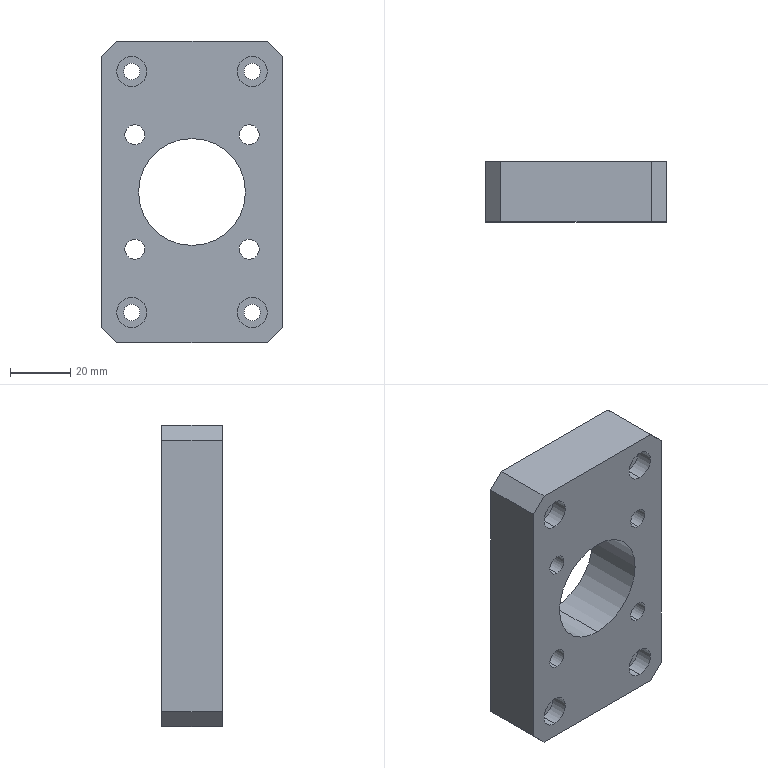Part | SolidWorks | features HoleWzd 2, Chamfer 1, Extrusion 1, ICE 1 | 1 solid | 52 faces | box 60 x 20 x 100 mm | volume 92174 mm3 | cylinder 34 | plane 18 | commonest cylinder face diameters 5.5 x8 6.6 x8 10 x8 11 x8 35.5 x2
STEP:
#1=CARTESIAN_POINT('',(-20.,5.7,-35.));
#2=VERTEX_POINT('',#1);
#3=CARTESIAN_POINT('',(-20.,5.7,-45.));
#4=VERTEX_POINT('',#3);
#5=CARTESIAN_POINT('',(-20.,5.7,-40.));
#6=DIRECTION('',(0.,-1.,0.));
#7=DIRECTION('',(0.,0.,-1.));
#8=AXIS2_PLACEMENT_3D('',#5,#6,#7);
#9=CIRCLE('',#8,5.);
#10=EDGE_CURVE('',#2,#4,#9,.T.);
#11=ORIENTED_EDGE('',*,*,#10,.F.);
#12=CARTESIAN_POINT('',(-20.,0.,-35.));
#13=VERTEX_POINT('',#12);
#14=CARTESIAN_POINT('',(-20.,0.,-35.));
#15=DIRECTION('',(0.,-1.,0.));
#16=VECTOR('',#15,1000.);
#17=LINE('',#14,#16);
#18=EDGE_CURVE('',#2,#13,#17,.T.);
#19=ORIENTED_EDGE('',*,*,#18,.T.);
#20=CARTESIAN_POINT('',(-20.,0.,-45.));
#21=VERTEX_POINT('',#20);
#22=CARTESIAN_POINT('',(-20.,0.,-40.));
#23=DIRECTION('',(0.,-1.,0.));
#24=DIRECTION('',(0.,0.,-1.));
#25=AXIS2_PLACEMENT_3D('',#22,#23,#24);
#26=CIRCLE('',#25,5.);
#27=EDGE_CURVE('',#13,#21,#26,.T.);
#28=ORIENTED_EDGE('',*,*,#27,.T.);
#29=CARTESIAN_POINT('',(-20.,0.,-45.));
#30=DIRECTION('',(0.,-1.,0.));
#31=VECTOR('',#30,1000.);
#32=LINE('',#29,#31);
#33=EDGE_CURVE('',#4,#21,#32,.T.);
#34=ORIENTED_EDGE('',*,*,#33,.F.);
#35=EDGE_LOOP('',(#11,#19,#28,#34));
#36=FACE_OUTER_BOUND('',#35,.T.);
#37=CARTESIAN_POINT('',(-20.,0.,-40.));
#38=DIRECTION('',(0.,-1.,0.));
#39=DIRECTION('',(0.,0.,-1.));
#40=AXIS2_PLACEMENT_3D('',#37,#38,#39);
#41=CYLINDRICAL_SURFACE('',#40,5.);
#42=ADVANCED_FACE('',(#36),#41,.F.);
#43=CARTESIAN_POINT('',(-20.,20.,-42.75));
#44=VERTEX_POINT('',#43);
#45=CARTESIAN_POINT('',(-20.,20.,-37.25));
#46=VERTEX_POINT('',#45);
#47=CARTESIAN_POINT('',(-20.,20.,-40.));
#48=DIRECTION('',(0.,1.,0.));
#49=DIRECTION('',(0.,0.,1.));
#50=AXIS2_PLACEMENT_3D('',#47,#48,#49);
#51=CIRCLE('',#50,2.75);
#52=EDGE_CURVE('',#44,#46,#51,.T.);
#53=ORIENTED_EDGE('',*,*,#52,.T.);
#54=CARTESIAN_POINT('',(-20.,5.7,-37.25));
#55=VERTEX_POINT('',#54);
#56=CARTESIAN_POINT('',(-20.,0.,-37.25));
#57=DIRECTION('',(0.,-1.,0.));
#58=VECTOR('',#57,1000.);
#59=LINE('',#56,#58);
#60=EDGE_CURVE('',#46,#55,#59,.T.);
#61=ORIENTED_EDGE('',*,*,#60,.T.);
#62=CARTESIAN_POINT('',(-20.,5.7,-42.75));
#63=VERTEX_POINT('',#62);
#64=CARTESIAN_POINT('',(-20.,5.7,-40.));
#65=DIRECTION('',(0.,-1.,0.));
#66=DIRECTION('',(0.,0.,-1.));
#67=AXIS2_PLACEMENT_3D('',#64,#65,#66);
#68=CIRCLE('',#67,2.75);
#69=EDGE_CURVE('',#55,#63,#68,.T.);
#70=ORIENTED_EDGE('',*,*,#69,.T.);
#71=CARTESIAN_POINT('',(-20.,0.,-42.75));
#72=DIRECTION('',(0.,-1.,0.));
#73=VECTOR('',#72,1000.);
#74=LINE('',#71,#73);
#75=EDGE_CURVE('',#44,#63,#74,.T.);
#76=ORIENTED_EDGE('',*,*,#75,.F.);
#77=EDGE_LOOP('',(#53,#61,#70,#76));
#78=FACE_OUTER_BOUND('',#77,.T.);
#79=CARTESIAN_POINT('',(-20.,0.,-40.));
#80=DIRECTION('',(0.,-1.,0.));
#81=DIRECTION('',(0.,0.,-1.));
#82=AXIS2_PLACEMENT_3D('',#79,#80,#81);
#83=CYLINDRICAL_SURFACE('',#82,2.75);
#84=ADVANCED_FACE('',(#78),#83,.F.);
#85=CARTESIAN_POINT('',(20.,5.7,-35.));
#86=VERTEX_POINT('',#85);
#87=CARTESIAN_POINT('',(20.,5.7,-45.));
#88=VERTEX_POINT('',#87);
#89=CARTESIAN_POINT('',(20.,5.7,-40.));
#90=DIRECTION('',(0.,-1.,0.));
#91=DIRECTION('',(0.,0.,-1.));
#92=AXIS2_PLACEMENT_3D('',#89,#90,#91);
#93=CIRCLE('',#92,5.);
#94=EDGE_CURVE('',#86,#88,#93,.T.);
#95=ORIENTED_EDGE('',*,*,#94,.F.);
#96=CARTESIAN_POINT('',(20.,0.,-35.));
#97=VERTEX_POINT('',#96);
#98=CARTESIAN_POINT('',(20.,0.,-35.));
#99=DIRECTION('',(0.,-1.,0.));
#100=VECTOR('',#99,1000.);
#101=LINE('',#98,#100);
#102=EDGE_CURVE('',#86,#97,#101,.T.);
#103=ORIENTED_EDGE('',*,*,#102,.T.);
#104=CARTESIAN_POINT('',(20.,0.,-45.));
#105=VERTEX_POINT('',#104);
#106=CARTESIAN_POINT('',(20.,0.,-40.));
#107=DIRECTION('',(0.,-1.,0.));
#108=DIRECTION('',(0.,0.,-1.));
#109=AXIS2_PLACEMENT_3D('',#106,#107,#108);
#110=CIRCLE('',#109,5.);
#111=EDGE_CURVE('',#97,#105,#110,.T.);
#112=ORIENTED_EDGE('',*,*,#111,.T.);
#113=CARTESIAN_POINT('',(20.,0.,-45.));
#114=DIRECTION('',(0.,-1.,0.));
#115=VECTOR('',#114,1000.);
#116=LINE('',#113,#115);
#117=EDGE_CURVE('',#88,#105,#116,.T.);
#118=ORIENTED_EDGE('',*,*,#117,.F.);
#119=EDGE_LOOP('',(#95,#103,#112,#118));
#120=FACE_OUTER_BOUND('',#119,.T.);
#121=CARTESIAN_POINT('',(20.,0.,-40.));
#122=DIRECTION('',(0.,-1.,0.));
#123=DIRECTION('',(0.,0.,-1.));
#124=AXIS2_PLACEMENT_3D('',#121,#122,#123);
#125=CYLINDRICAL_SURFACE('',#124,5.);
#126=ADVANCED_FACE('',(#120),#125,.F.);
#127=CARTESIAN_POINT('',(20.,20.,-42.75));
#128=VERTEX_POINT('',#127);
#129=CARTESIAN_POINT('',(20.,20.,-37.25));
#130=VERTEX_POINT('',#129);
#131=CARTESIAN_POINT('',(20.,20.,-40.));
#132=DIRECTION('',(0.,1.,0.));
#133=DIRECTION('',(0.,0.,1.));
#134=AXIS2_PLACEMENT_3D('',#131,#132,#133);
#135=CIRCLE('',#134,2.75);
#136=EDGE_CURVE('',#128,#130,#135,.T.);
#137=ORIENTED_EDGE('',*,*,#136,.T.);
#138=CARTESIAN_POINT('',(20.,5.7,-37.25));
#139=VERTEX_POINT('',#138);
#140=CARTESIAN_POINT('',(20.,0.,-37.25));
#141=DIRECTION('',(0.,-1.,0.));
#142=VECTOR('',#141,1000.);
#143=LINE('',#140,#142);
#144=EDGE_CURVE('',#130,#139,#143,.T.);
#145=ORIENTED_EDGE('',*,*,#144,.T.);
#146=CARTESIAN_POINT('',(20.,5.7,-42.75));
#147=VERTEX_POINT('',#146);
#148=CARTESIAN_POINT('',(20.,5.7,-40.));
#149=DIRECTION('',(0.,-1.,0.));
#150=DIRECTION('',(0.,0.,-1.));
#151=AXIS2_PLACEMENT_3D('',#148,#149,#150);
#152=CIRCLE('',#151,2.75);
#153=EDGE_CURVE('',#139,#147,#152,.T.);
#154=ORIENTED_EDGE('',*,*,#153,.T.);
#155=CARTESIAN_POINT('',(20.,0.,-42.75));
#156=DIRECTION('',(0.,-1.,0.));
#157=VECTOR('',#156,1000.);
#158=LINE('',#155,#157);
#159=EDGE_CURVE('',#128,#147,#158,.T.);
#160=ORIENTED_EDGE('',*,*,#159,.F.);
#161=EDGE_LOOP('',(#137,#145,#154,#160));
#162=FACE_OUTER_BOUND('',#161,.T.);
#163=CARTESIAN_POINT('',(20.,0.,-40.));
#164=DIRECTION('',(0.,-1.,0.));
#165=DIRECTION('',(0.,0.,-1.));
#166=AXIS2_PLACEMENT_3D('',#163,#164,#165);
#167=CYLINDRICAL_SURFACE('',#166,2.75);
#168=ADVANCED_FACE('',(#162),#167,.F.);
#169=CARTESIAN_POINT('',(-20.,5.7,45.));
#170=VERTEX_POINT('',#169);
#171=CARTESIAN_POINT('',(-20.,5.7,35.));
#172=VERTEX_POINT('',#171);
#173=CARTESIAN_POINT('',(-20.,5.7,40.));
#174=DIRECTION('',(0.,-1.,0.));
#175=DIRECTION('',(0.,0.,-1.));
#176=AXIS2_PLACEMENT_3D('',#173,#174,#175);
#177=CIRCLE('',#176,5.);
#178=EDGE_CURVE('',#170,#172,#177,.T.);
#179=ORIENTED_EDGE('',*,*,#178,.F.);
#180=CARTESIAN_POINT('',(-20.,0.,45.));
#181=VERTEX_POINT('',#180);
#182=CARTESIAN_POINT('',(-20.,0.,45.));
#183=DIRECTION('',(0.,-1.,0.));
#184=VECTOR('',#183,1000.);
#185=LINE('',#182,#184);
#186=EDGE_CURVE('',#170,#181,#185,.T.);
#187=ORIENTED_EDGE('',*,*,#186,.T.);
#188=CARTESIAN_POINT('',(-20.,0.,35.));
#189=VERTEX_POINT('',#188);
#190=CARTESIAN_POINT('',(-20.,0.,40.));
#191=DIRECTION('',(0.,-1.,0.));
#192=DIRECTION('',(0.,0.,-1.));
#193=AXIS2_PLACEMENT_3D('',#190,#191,#192);
#194=CIRCLE('',#193,5.);
#195=EDGE_CURVE('',#181,#189,#194,.T.);
#196=ORIENTED_EDGE('',*,*,#195,.T.);
#197=CARTESIAN_POINT('',(-20.,0.,35.));
#198=DIRECTION('',(0.,-1.,0.));
#199=VECTOR('',#198,1000.);
#200=LINE('',#197,#199);
#201=EDGE_CURVE('',#172,#189,#200,.T.);
#202=ORIENTED_EDGE('',*,*,#201,.F.);
#203=EDGE_LOOP('',(#179,#187,#196,#202));
#204=FACE_OUTER_BOUND('',#203,.T.);
#205=CARTESIAN_POINT('',(-20.,0.,40.));
#206=DIRECTION('',(0.,-1.,0.));
#207=DIRECTION('',(0.,0.,-1.));
#208=AXIS2_PLACEMENT_3D('',#205,#206,#207);
#209=CYLINDRICAL_SURFACE('',#208,5.);
#210=ADVANCED_FACE('',(#204),#209,.F.);
#211=CARTESIAN_POINT('',(-20.,20.,37.25));
#212=VERTEX_POINT('',#211);
#213=CARTESIAN_POINT('',(-20.,20.,42.75));
#214=VERTEX_POINT('',#213);
#215=CARTESIAN_POINT('',(-20.,20.,40.));
#216=DIRECTION('',(0.,1.,0.));
#217=DIRECTION('',(0.,0.,1.));
#218=AXIS2_PLACEMENT_3D('',#215,#216,#217);
#219=CIRCLE('',#218,2.75);
#220=EDGE_CURVE('',#212,#214,#219,.T.);
#221=ORIENTED_EDGE('',*,*,#220,.T.);
#222=CARTESIAN_POINT('',(-20.,5.7,42.75));
#223=VERTEX_POINT('',#222);
#224=CARTESIAN_POINT('',(-20.,0.,42.75));
#225=DIRECTION('',(0.,-1.,0.));
#226=VECTOR('',#225,1000.);
#227=LINE('',#224,#226);
#228=EDGE_CURVE('',#214,#223,#227,.T.);
#229=ORIENTED_EDGE('',*,*,#228,.T.);
#230=CARTESIAN_POINT('',(-20.,5.7,37.25));
#231=VERTEX_POINT('',#230);
#232=CARTESIAN_POINT('',(-20.,5.7,40.));
#233=DIRECTION('',(0.,-1.,0.));
#234=DIRECTION('',(0.,0.,-1.));
#235=AXIS2_PLACEMENT_3D('',#232,#233,#234);
#236=CIRCLE('',#235,2.75);
#237=EDGE_CURVE('',#223,#231,#236,.T.);
#238=ORIENTED_EDGE('',*,*,#237,.T.);
#239=CARTESIAN_POINT('',(-20.,0.,37.25));
#240=DIRECTION('',(0.,-1.,0.));
#241=VECTOR('',#240,1000.);
#242=LINE('',#239,#241);
#243=EDGE_CURVE('',#212,#231,#242,.T.);
#244=ORIENTED_EDGE('',*,*,#243,.F.);
#245=EDGE_LOOP('',(#221,#229,#238,#244));
#246=FACE_OUTER_BOUND('',#245,.T.);
#247=CARTESIAN_POINT('',(-20.,0.,40.));
#248=DIRECTION('',(0.,-1.,0.));
#249=DIRECTION('',(0.,0.,-1.));
#250=AXIS2_PLACEMENT_3D('',#247,#248,#249);
#251=CYLINDRICAL_SURFACE('',#250,2.75);
#252=ADVANCED_FACE('',(#246),#251,.F.);
#253=CARTESIAN_POINT('',(20.,5.7,45.));
#254=VERTEX_POINT('',#253);
#255=CARTESIAN_POINT('',(20.,5.7,35.));
#256=VERTEX_POINT('',#255);
#257=CARTESIAN_POINT('',(20.,5.7,40.));
#258=DIRECTION('',(0.,-1.,0.));
#259=DIRECTION('',(0.,0.,-1.));
#260=AXIS2_PLACEMENT_3D('',#257,#258,#259);
#261=CIRCLE('',#260,5.);
#262=EDGE_CURVE('',#254,#256,#261,.T.);
#263=ORIENTED_EDGE('',*,*,#262,.F.);
#264=CARTESIAN_POINT('',(20.,0.,45.));
#265=VERTEX_POINT('',#264);
#266=CARTESIAN_POINT('',(20.,0.,45.));
#267=DIRECTION('',(0.,-1.,0.));
#268=VECTOR('',#267,1000.);
#269=LINE('',#266,#268);
#270=EDGE_CURVE('',#254,#265,#269,.T.);
#271=ORIENTED_EDGE('',*,*,#270,.T.);
#272=CARTESIAN_POINT('',(20.,0.,35.));
#273=VERTEX_POINT('',#272);
#274=CARTESIAN_POINT('',(20.,0.,40.));
#275=DIRECTION('',(0.,-1.,0.));
#276=DIRECTION('',(0.,0.,-1.));
#277=AXIS2_PLACEMENT_3D('',#274,#275,#276);
#278=CIRCLE('',#277,5.);
#279=EDGE_CURVE('',#265,#273,#278,.T.);
#280=ORIENTED_EDGE('',*,*,#279,.T.);
#281=CARTESIAN_POINT('',(20.,0.,35.));
#282=DIRECTION('',(0.,-1.,0.));
#283=VECTOR('',#282,1000.);
#284=LINE('',#281,#283);
#285=EDGE_CURVE('',#256,#273,#284,.T.);
#286=ORIENTED_EDGE('',*,*,#285,.F.);
#287=EDGE_LOOP('',(#263,#271,#280,#286));
#288=FACE_OUTER_BOUND('',#287,.T.);
#289=CARTESIAN_POINT('',(20.,0.,40.));
#290=DIRECTION('',(0.,-1.,0.));
#291=DIRECTION('',(0.,0.,-1.));
#292=AXIS2_PLACEMENT_3D('',#289,#290,#291);
#293=CYLINDRICAL_SURFACE('',#292,5.);
#294=ADVANCED_FACE('',(#288),#293,.F.);
#295=CARTESIAN_POINT('',(20.,20.,37.25));
#296=VERTEX_POINT('',#295);
#297=CARTESIAN_POINT('',(20.,20.,42.75));
#298=VERTEX_POINT('',#297);
#299=CARTESIAN_POINT('',(20.,20.,40.));
#300=DIRECTION('',(0.,1.,0.));
#301=DIRECTION('',(0.,0.,1.));
#302=AXIS2_PLACEMENT_3D('',#299,#300,#301);
#303=CIRCLE('',#302,2.75);
#304=EDGE_CURVE('',#296,#298,#303,.T.);
#305=ORIENTED_EDGE('',*,*,#304,.T.);
#306=CARTESIAN_POINT('',(20.,5.7,42.75));
#307=VERTEX_POINT('',#306);
#308=CARTESIAN_POINT('',(20.,0.,42.75));
#309=DIRECTION('',(0.,-1.,0.));
#310=VECTOR('',#309,1000.);
#311=LINE('',#308,#310);
#312=EDGE_CURVE('',#298,#307,#311,.T.);
#313=ORIENTED_EDGE('',*,*,#312,.T.);
#314=CARTESIAN_POINT('',(20.,5.7,37.25));
#315=VERTEX_POINT('',#314);
#316=CARTESIAN_POINT('',(20.,5.7,40.));
#317=DIRECTION('',(0.,-1.,0.));
#318=DIRECTION('',(0.,0.,-1.));
#319=AXIS2_PLACEMENT_3D('',#316,#317,#318);
#320=CIRCLE('',#319,2.75);
#321=EDGE_CURVE('',#307,#315,#320,.T.);
#322=ORIENTED_EDGE('',*,*,#321,.T.);
#323=CARTESIAN_POINT('',(20.,0.,37.25));
#324=DIRECTION('',(0.,-1.,0.));
#325=VECTOR('',#324,1000.);
#326=LINE('',#323,#325);
#327=EDGE_CURVE('',#296,#315,#326,.T.);
#328=ORIENTED_EDGE('',*,*,#327,.F.);
#329=EDGE_LOOP('',(#305,#313,#322,#328));
#330=FACE_OUTER_BOUND('',#329,.T.);
#331=CARTESIAN_POINT('',(20.,0.,40.));
#332=DIRECTION('',(0.,-1.,0.));
#333=DIRECTION('',(0.,0.,-1.));
#334=AXIS2_PLACEMENT_3D('',#331,#332,#333);
#335=CYLINDRICAL_SURFACE('',#334,2.75);
#336=ADVANCED_FACE('',(#330),#335,.F.);
#337=CARTESIAN_POINT('',(19.,15.3,-24.5));
#338=VERTEX_POINT('',#337);
#339=CARTESIAN_POINT('',(19.,15.3,-13.5));
#340=VERTEX_POINT('',#339);
#341=CARTESIAN_POINT('',(19.,15.3,-19.));
#342=DIRECTION('',(0.,1.,0.));
#343=DIRECTION('',(0.,0.,1.));
#344=AXIS2_PLACEMENT_3D('',#341,#342,#343);
#345=CIRCLE('',#344,5.5);
#346=EDGE_CURVE('',#338,#340,#345,.T.);
#347=ORIENTED_EDGE('',*,*,#346,.F.);
#348=CARTESIAN_POINT('',(19.,20.,-24.5));
#349=VERTEX_POINT('',#348);
#350=CARTESIAN_POINT('',(19.,20.,-24.5));
#351=DIRECTION('',(0.,1.,0.));
#352=VECTOR('',#351,1000.);
#353=LINE('',#350,#352);
#354=EDGE_CURVE('',#338,#349,#353,.T.);
#355=ORIENTED_EDGE('',*,*,#354,.T.);
#356=CARTESIAN_POINT('',(19.,20.,-13.5));
#357=VERTEX_POINT('',#356);
#358=CARTESIAN_POINT('',(19.,20.,-19.));
#359=DIRECTION('',(0.,1.,0.));
#360=DIRECTION('',(0.,0.,1.));
#361=AXIS2_PLACEMENT_3D('',#358,#359,#360);
#362=CIRCLE('',#361,5.5);
#363=EDGE_CURVE('',#349,#357,#362,.T.);
#364=ORIENTED_EDGE('',*,*,#363,.T.);
#365=CARTESIAN_POINT('',(19.,20.,-13.5));
#366=DIRECTION('',(0.,1.,0.));
#367=VECTOR('',#366,1000.);
#368=LINE('',#365,#367);
#369=EDGE_CURVE('',#340,#357,#368,.T.);
#370=ORIENTED_EDGE('',*,*,#369,.F.);
#371=EDGE_LOOP('',(#347,#355,#364,#370));
#372=FACE_OUTER_BOUND('',#371,.T.);
#373=CARTESIAN_POINT('',(19.,20.,-19.));
#374=DIRECTION('',(0.,1.,0.));
#375=DIRECTION('',(0.,0.,1.));
#376=AXIS2_PLACEMENT_3D('',#373,#374,#375);
#377=CYLINDRICAL_SURFACE('',#376,5.5);
#378=ADVANCED_FACE('',(#372),#377,.F.);
#379=CARTESIAN_POINT('',(19.,0.,-22.3));
#380=VERTEX_POINT('',#379);
#381=CARTESIAN_POINT('',(19.,0.,-15.7));
#382=VERTEX_POINT('',#381);
#383=CARTESIAN_POINT('',(19.,0.,-19.));
#384=DIRECTION('',(0.,1.,0.));
#385=DIRECTION('',(0.,0.,1.));
#386=AXIS2_PLACEMENT_3D('',#383,#384,#385);
#387=CIRCLE('',#386,3.3);
#388=EDGE_CURVE('',#380,#382,#387,.T.);
#389=ORIENTED_EDGE('',*,*,#388,.F.);
#390=CARTESIAN_POINT('',(19.,15.3,-22.3));
#391=VERTEX_POINT('',#390);
#392=CARTESIAN_POINT('',(19.,20.,-22.3));
#393=DIRECTION('',(0.,1.,0.));
#394=VECTOR('',#393,1000.);
#395=LINE('',#392,#394);
#396=EDGE_CURVE('',#380,#391,#395,.T.);
#397=ORIENTED_EDGE('',*,*,#396,.T.);
#398=CARTESIAN_POINT('',(19.,15.3,-15.7));
#399=VERTEX_POINT('',#398);
#400=CARTESIAN_POINT('',(19.,15.3,-19.));
#401=DIRECTION('',(0.,1.,0.));
#402=DIRECTION('',(0.,0.,1.));
#403=AXIS2_PLACEMENT_3D('',#400,#401,#402);
#404=CIRCLE('',#403,3.3);
#405=EDGE_CURVE('',#391,#399,#404,.T.);
#406=ORIENTED_EDGE('',*,*,#405,.T.);
#407=CARTESIAN_POINT('',(19.,20.,-15.7));
#408=DIRECTION('',(0.,1.,0.));
#409=VECTOR('',#408,1000.);
#410=LINE('',#407,#409);
#411=EDGE_CURVE('',#382,#399,#410,.T.);
#412=ORIENTED_EDGE('',*,*,#411,.F.);
#413=EDGE_LOOP('',(#389,#397,#406,#412));
#414=FACE_OUTER_BOUND('',#413,.T.);
#415=CARTESIAN_POINT('',(19.,20.,-19.));
#416=DIRECTION('',(0.,1.,0.));
#417=DIRECTION('',(0.,0.,1.));
#418=AXIS2_PLACEMENT_3D('',#415,#416,#417);
#419=CYLINDRICAL_SURFACE('',#418,3.3);
#420=ADVANCED_FACE('',(#414),#419,.F.);
#421=CARTESIAN_POINT('',(19.,15.3,13.5));
#422=VERTEX_POINT('',#421);
#423=CARTESIAN_POINT('',(19.,15.3,24.5));
#424=VERTEX_POINT('',#423);
#425=CARTESIAN_POINT('',(19.,15.3,19.));
#426=DIRECTION('',(0.,1.,0.));
#427=DIRECTION('',(0.,0.,1.));
#428=AXIS2_PLACEMENT_3D('',#425,#426,#427);
#429=CIRCLE('',#428,5.5);
#430=EDGE_CURVE('',#422,#424,#429,.T.);
#431=ORIENTED_EDGE('',*,*,#430,.F.);
#432=CARTESIAN_POINT('',(19.,20.,13.5));
#433=VERTEX_POINT('',#432);
#434=CARTESIAN_POINT('',(19.,20.,13.5));
#435=DIRECTION('',(0.,1.,0.));
#436=VECTOR('',#435,1000.);
#437=LINE('',#434,#436);
#438=EDGE_CURVE('',#422,#433,#437,.T.);
#439=ORIENTED_EDGE('',*,*,#438,.T.);
#440=CARTESIAN_POINT('',(19.,20.,24.5));
#441=VERTEX_POINT('',#440);
#442=CARTESIAN_POINT('',(19.,20.,19.));
#443=DIRECTION('',(0.,1.,0.));
#444=DIRECTION('',(0.,0.,1.));
#445=AXIS2_PLACEMENT_3D('',#442,#443,#444);
#446=CIRCLE('',#445,5.5);
#447=EDGE_CURVE('',#433,#441,#446,.T.);
#448=ORIENTED_EDGE('',*,*,#447,.T.);
#449=CARTESIAN_POINT('',(19.,20.,24.5));
#450=DIRECTION('',(0.,1.,0.));
#451=VECTOR('',#450,1000.);
#452=LINE('',#449,#451);
#453=EDGE_CURVE('',#424,#441,#452,.T.);
#454=ORIENTED_EDGE('',*,*,#453,.F.);
#455=EDGE_LOOP('',(#431,#439,#448,#454));
#456=FACE_OUTER_BOUND('',#455,.T.);
#457=CARTESIAN_POINT('',(19.,20.,19.));
#458=DIRECTION('',(0.,1.,0.));
#459=DIRECTION('',(0.,0.,1.));
#460=AXIS2_PLACEMENT_3D('',#457,#458,#459);
#461=CYLINDRICAL_SURFACE('',#460,5.5);
#462=ADVANCED_FACE('',(#456),#461,.F.);
#463=CARTESIAN_POINT('',(19.,0.,15.7));
#464=VERTEX_POINT('',#463);
#465=CARTESIAN_POINT('',(19.,0.,22.3));
#466=VERTEX_POINT('',#465);
#467=CARTESIAN_POINT('',(19.,0.,19.));
#468=DIRECTION('',(0.,1.,0.));
#469=DIRECTION('',(0.,0.,1.));
#470=AXIS2_PLACEMENT_3D('',#467,#468,#469);
#471=CIRCLE('',#470,3.3);
#472=EDGE_CURVE('',#464,#466,#471,.T.);
#473=ORIENTED_EDGE('',*,*,#472,.F.);
#474=CARTESIAN_POINT('',(19.,15.3,15.7));
#475=VERTEX_POINT('',#474);
#476=CARTESIAN_POINT('',(19.,20.,15.7));
#477=DIRECTION('',(0.,1.,0.));
#478=VECTOR('',#477,1000.);
#479=LINE('',#476,#478);
#480=EDGE_CURVE('',#464,#475,#479,.T.);
#481=ORIENTED_EDGE('',*,*,#480,.T.);
#482=CARTESIAN_POINT('',(19.,15.3,22.3));
#483=VERTEX_POINT('',#482);
#484=CARTESIAN_POINT('',(19.,15.3,19.));
#485=DIRECTION('',(0.,1.,0.));
#486=DIRECTION('',(0.,0.,1.));
#487=AXIS2_PLACEMENT_3D('',#484,#485,#486);
#488=CIRCLE('',#487,3.3);
#489=EDGE_CURVE('',#475,#483,#488,.T.);
#490=ORIENTED_EDGE('',*,*,#489,.T.);
#491=CARTESIAN_POINT('',(19.,20.,22.3));
#492=DIRECTION('',(0.,1.,0.));
#493=VECTOR('',#492,1000.);
#494=LINE('',#491,#493);
#495=EDGE_CURVE('',#466,#483,#494,.T.);
#496=ORIENTED_EDGE('',*,*,#495,.F.);
#497=EDGE_LOOP('',(#473,#481,#490,#496));
#498=FACE_OUTER_BOUND('',#497,.T.);
#499=CARTESIAN_POINT('',(19.,20.,19.));
#500=DIRECTION('',(0.,1.,0.));
#501=DIRECTION('',(0.,0.,1.));
#502=AXIS2_PLACEMENT_3D('',#499,#500,#501);
#503=CYLINDRICAL_SURFACE('',#502,3.3);
#504=ADVANCED_FACE('',(#498),#503,.F.);
#505=CARTESIAN_POINT('',(-19.,15.3,-24.5));
#506=VERTEX_POINT('',#505);
#507=CARTESIAN_POINT('',(-19.,15.3,-13.5));
#508=VERTEX_POINT('',#507);
#509=CARTESIAN_POINT('',(-19.,15.3,-19.));
#510=DIRECTION('',(0.,1.,0.));
#511=DIRECTION('',(0.,0.,1.));
#512=AXIS2_PLACEMENT_3D('',#509,#510,#511);
#513=CIRCLE('',#512,5.5);
#514=EDGE_CURVE('',#506,#508,#513,.T.);
#515=ORIENTED_EDGE('',*,*,#514,.F.);
#516=CARTESIAN_POINT('',(-19.,20.,-24.5));
#517=VERTEX_POINT('',#516);
#518=CARTESIAN_POINT('',(-19.,20.,-24.5));
#519=DIRECTION('',(0.,1.,0.));
#520=VECTOR('',#519,1000.);
#521=LINE('',#518,#520);
#522=EDGE_CURVE('',#506,#517,#521,.T.);
#523=ORIENTED_EDGE('',*,*,#522,.T.);
#524=CARTESIAN_POINT('',(-19.,20.,-13.5));
#525=VERTEX_POINT('',#524);
#526=CARTESIAN_POINT('',(-19.,20.,-19.));
#527=DIRECTION('',(0.,1.,0.));
#528=DIRECTION('',(0.,0.,1.));
#529=AXIS2_PLACEMENT_3D('',#526,#527,#528);
#530=CIRCLE('',#529,5.5);
#531=EDGE_CURVE('',#517,#525,#530,.T.);
#532=ORIENTED_EDGE('',*,*,#531,.T.);
#533=CARTESIAN_POINT('',(-19.,20.,-13.5));
#534=DIRECTION('',(0.,1.,0.));
#535=VECTOR('',#534,1000.);
#536=LINE('',#533,#535);
#537=EDGE_CURVE('',#508,#525,#536,.T.);
#538=ORIENTED_EDGE('',*,*,#537,.F.);
#539=EDGE_LOOP('',(#515,#523,#532,#538));
#540=FACE_OUTER_BOUND('',#539,.T.);
#541=CARTESIAN_POINT('',(-19.,20.,-19.));
#542=DIRECTION('',(0.,1.,0.));
#543=DIRECTION('',(0.,0.,1.));
#544=AXIS2_PLACEMENT_3D('',#541,#542,#543);
#545=CYLINDRICAL_SURFACE('',#544,5.5);
#546=ADVANCED_FACE('',(#540),#545,.F.);
#547=CARTESIAN_POINT('',(-19.,0.,-22.3));
#548=VERTEX_POINT('',#547);
#549=CARTESIAN_POINT('',(-19.,0.,-15.7));
#550=VERTEX_POINT('',#549);
#551=CARTESIAN_POINT('',(-19.,0.,-19.));
#552=DIRECTION('',(0.,1.,0.));
#553=DIRECTION('',(0.,0.,1.));
#554=AXIS2_PLACEMENT_3D('',#551,#552,#553);
#555=CIRCLE('',#554,3.3);
#556=EDGE_CURVE('',#548,#550,#555,.T.);
#557=ORIENTED_EDGE('',*,*,#556,.F.);
#558=CARTESIAN_POINT('',(-19.,15.3,-22.3));
#559=VERTEX_POINT('',#558);
#560=CARTESIAN_POINT('',(-19.,20.,-22.3));
#561=DIRECTION('',(0.,1.,0.));
#562=VECTOR('',#561,1000.);
#563=LINE('',#560,#562);
#564=EDGE_CURVE('',#548,#559,#563,.T.);
#565=ORIENTED_EDGE('',*,*,#564,.T.);
#566=CARTESIAN_POINT('',(-19.,15.3,-15.7));
#567=VERTEX_POINT('',#566);
#568=CARTESIAN_POINT('',(-19.,15.3,-19.));
#569=DIRECTION('',(0.,1.,0.));
#570=DIRECTION('',(0.,0.,1.));
#571=AXIS2_PLACEMENT_3D('',#568,#569,#570);
#572=CIRCLE('',#571,3.3);
#573=EDGE_CURVE('',#559,#567,#572,.T.);
#574=ORIENTED_EDGE('',*,*,#573,.T.);
#575=CARTESIAN_POINT('',(-19.,20.,-15.7));
#576=DIRECTION('',(0.,1.,0.));
#577=VECTOR('',#576,1000.);
#578=LINE('',#575,#577);
#579=EDGE_CURVE('',#550,#567,#578,.T.);
#580=ORIENTED_EDGE('',*,*,#579,.F.);
#581=EDGE_LOOP('',(#557,#565,#574,#580));
#582=FACE_OUTER_BOUND('',#581,.T.);
#583=CARTESIAN_POINT('',(-19.,20.,-19.));
#584=DIRECTION('',(0.,1.,0.));
#585=DIRECTION('',(0.,0.,1.));
#586=AXIS2_PLACEMENT_3D('',#583,#584,#585);
#587=CYLINDRICAL_SURFACE('',#586,3.3);
#588=ADVANCED_FACE('',(#582),#587,.F.);
#589=CARTESIAN_POINT('',(-19.,15.3,13.5));
#590=VERTEX_POINT('',#589);
#591=CARTESIAN_POINT('',(-19.,15.3,24.5));
#592=VERTEX_POINT('',#591);
#593=CARTESIAN_POINT('',(-19.,15.3,19.));
#594=DIRECTION('',(0.,1.,0.));
#595=DIRECTION('',(0.,0.,1.));
#596=AXIS2_PLACEMENT_3D('',#593,#594,#595);
#597=CIRCLE('',#596,5.5);
#598=EDGE_CURVE('',#590,#592,#597,.T.);
#599=ORIENTED_EDGE('',*,*,#598,.F.);
#600=CARTESIAN_POINT('',(-19.,20.,13.5));
#601=VERTEX_POINT('',#600);
#602=CARTESIAN_POINT('',(-19.,20.,13.5));
#603=DIRECTION('',(0.,1.,0.));
#604=VECTOR('',#603,1000.);
#605=LINE('',#602,#604);
#606=EDGE_CURVE('',#590,#601,#605,.T.);
#607=ORIENTED_EDGE('',*,*,#606,.T.);
#608=CARTESIAN_POINT('',(-19.,20.,24.5));
#609=VERTEX_POINT('',#608);
#610=CARTESIAN_POINT('',(-19.,20.,19.));
#611=DIRECTION('',(0.,1.,0.));
#612=DIRECTION('',(0.,0.,1.));
#613=AXIS2_PLACEMENT_3D('',#610,#611,#612);
#614=CIRCLE('',#613,5.5);
#615=EDGE_CURVE('',#601,#609,#614,.T.);
#616=ORIENTED_EDGE('',*,*,#615,.T.);
#617=CARTESIAN_POINT('',(-19.,20.,24.5));
#618=DIRECTION('',(0.,1.,0.));
#619=VECTOR('',#618,1000.);
#620=LINE('',#617,#619);
#621=EDGE_CURVE('',#592,#609,#620,.T.);
#622=ORIENTED_EDGE('',*,*,#621,.F.);
#623=EDGE_LOOP('',(#599,#607,#616,#622));
#624=FACE_OUTER_BOUND('',#623,.T.);
#625=CARTESIAN_POINT('',(-19.,20.,19.));
#626=DIRECTION('',(0.,1.,0.));
#627=DIRECTION('',(0.,0.,1.));
#628=AXIS2_PLACEMENT_3D('',#625,#626,#627);
#629=CYLINDRICAL_SURFACE('',#628,5.5);
#630=ADVANCED_FACE('',(#624),#629,.F.);
#631=CARTESIAN_POINT('',(-19.,0.,15.7));
#632=VERTEX_POINT('',#631);
#633=CARTESIAN_POINT('',(-19.,0.,22.3));
#634=VERTEX_POINT('',#633);
#635=CARTESIAN_POINT('',(-19.,0.,19.));
#636=DIRECTION('',(0.,1.,0.));
#637=DIRECTION('',(0.,0.,1.));
#638=AXIS2_PLACEMENT_3D('',#635,#636,#637);
#639=CIRCLE('',#638,3.3);
#640=EDGE_CURVE('',#632,#634,#639,.T.);
#641=ORIENTED_EDGE('',*,*,#640,.F.);
#642=CARTESIAN_POINT('',(-19.,15.3,15.7));
#643=VERTEX_POINT('',#642);
#644=CARTESIAN_POINT('',(-19.,20.,15.7));
#645=DIRECTION('',(0.,1.,0.));
#646=VECTOR('',#645,1000.);
#647=LINE('',#644,#646);
#648=EDGE_CURVE('',#632,#643,#647,.T.);
#649=ORIENTED_EDGE('',*,*,#648,.T.);
#650=CARTESIAN_POINT('',(-19.,15.3,22.3));
#651=VERTEX_POINT('',#650);
#652=CARTESIAN_POINT('',(-19.,15.3,19.));
#653=DIRECTION('',(0.,1.,0.));
#654=DIRECTION('',(0.,0.,1.));
#655=AXIS2_PLACEMENT_3D('',#652,#653,#654);
#656=CIRCLE('',#655,3.3);
#657=EDGE_CURVE('',#643,#651,#656,.T.);
#658=ORIENTED_EDGE('',*,*,#657,.T.);
#659=CARTESIAN_POINT('',(-19.,20.,22.3));
#660=DIRECTION('',(0.,1.,0.));
#661=VECTOR('',#660,1000.);
#662=LINE('',#659,#661);
#663=EDGE_CURVE('',#634,#651,#662,.T.);
#664=ORIENTED_EDGE('',*,*,#663,.F.);
#665=EDGE_LOOP('',(#641,#649,#658,#664));
#666=FACE_OUTER_BOUND('',#665,.T.);
#667=CARTESIAN_POINT('',(-19.,20.,19.));
#668=DIRECTION('',(0.,1.,0.));
#669=DIRECTION('',(0.,0.,1.));
#670=AXIS2_PLACEMENT_3D('',#667,#668,#669);
#671=CYLINDRICAL_SURFACE('',#670,3.3);
#672=ADVANCED_FACE('',(#666),#671,.F.);
#673=CARTESIAN_POINT('',(0.,0.,-17.75));
#674=VERTEX_POINT('',#673);
#675=CARTESIAN_POINT('',(0.,0.,17.75));
#676=VERTEX_POINT('',#675);
#677=CARTESIAN_POINT('',(0.,0.,0.));
#678=DIRECTION('',(0.,1.,0.));
#679=DIRECTION('',(0.,0.,1.));
#680=AXIS2_PLACEMENT_3D('',#677,#678,#679);
#681=CIRCLE('',#680,17.75);
#682=EDGE_CURVE('',#674,#676,#681,.T.);
#683=ORIENTED_EDGE('',*,*,#682,.F.);
#684=CARTESIAN_POINT('',(0.,20.,-17.75));
#685=VERTEX_POINT('',#684);
#686=CARTESIAN_POINT('',(0.,0.,-17.75));
#687=DIRECTION('',(0.,1.,0.));
#688=VECTOR('',#687,1000.);
#689=LINE('',#686,#688);
#690=EDGE_CURVE('',#674,#685,#689,.T.);
#691=ORIENTED_EDGE('',*,*,#690,.T.);
#692=CARTESIAN_POINT('',(0.,20.,17.75));
#693=VERTEX_POINT('',#692);
#694=CARTESIAN_POINT('',(0.,20.,0.));
#695=DIRECTION('',(0.,1.,0.));
#696=DIRECTION('',(0.,0.,1.));
#697=AXIS2_PLACEMENT_3D('',#694,#695,#696);
#698=CIRCLE('',#697,17.75);
#699=EDGE_CURVE('',#685,#693,#698,.T.);
#700=ORIENTED_EDGE('',*,*,#699,.T.);
#701=CARTESIAN_POINT('',(0.,0.,17.75));
#702=DIRECTION('',(0.,1.,0.));
#703=VECTOR('',#702,1000.);
#704=LINE('',#701,#703);
#705=EDGE_CURVE('',#676,#693,#704,.T.);
#706=ORIENTED_EDGE('',*,*,#705,.F.);
#707=EDGE_LOOP('',(#683,#691,#700,#706));
#708=FACE_OUTER_BOUND('',#707,.T.);
#709=CARTESIAN_POINT('',(0.,0.,0.));
#710=DIRECTION('',(0.,1.,0.));
#711=DIRECTION('',(0.,0.,1.));
#712=AXIS2_PLACEMENT_3D('',#709,#710,#711);
#713=CYLINDRICAL_SURFACE('',#712,17.75);
#714=ADVANCED_FACE('',(#708),#713,.F.);
#715=CARTESIAN_POINT('',(30.,20.,45.));
#716=VERTEX_POINT('',#715);
#717=CARTESIAN_POINT('',(30.,20.,-45.));
#718=VERTEX_POINT('',#717);
#719=CARTESIAN_POINT('',(30.,20.,-50.));
#720=DIRECTION('',(0.,0.,-1.));
#721=VECTOR('',#720,1000.);
#722=LINE('',#719,#721);
#723=EDGE_CURVE('',#716,#718,#722,.T.);
#724=ORIENTED_EDGE('',*,*,#723,.F.);
#725=CARTESIAN_POINT('',(30.,0.,45.));
#726=VERTEX_POINT('',#725);
#727=CARTESIAN_POINT('',(30.,20.,45.));
#728=DIRECTION('',(0.,-1.,0.));
#729=VECTOR('',#728,1000.);
#730=LINE('',#727,#729);
#731=EDGE_CURVE('',#716,#726,#730,.T.);
#732=ORIENTED_EDGE('',*,*,#731,.T.);
#733=CARTESIAN_POINT('',(30.,0.,-45.));
#734=VERTEX_POINT('',#733);
#735=CARTESIAN_POINT('',(30.,0.,-50.));
#736=DIRECTION('',(0.,0.,-1.));
#737=VECTOR('',#736,1000.);
#738=LINE('',#735,#737);
#739=EDGE_CURVE('',#726,#734,#738,.T.);
#740=ORIENTED_EDGE('',*,*,#739,.T.);
#741=CARTESIAN_POINT('',(30.,20.,-45.));
#742=DIRECTION('',(0.,1.,0.));
#743=VECTOR('',#742,1000.);
#744=LINE('',#741,#743);
#745=EDGE_CURVE('',#734,#718,#744,.T.);
#746=ORIENTED_EDGE('',*,*,#745,.T.);
#747=EDGE_LOOP('',(#724,#732,#740,#746));
#748=FACE_OUTER_BOUND('',#747,.T.);
#749=CARTESIAN_POINT('',(30.,20.,-50.));
#750=DIRECTION('',(-1.,0.,0.));
#751=DIRECTION('',(0.,0.,1.));
#752=AXIS2_PLACEMENT_3D('',#749,#750,#751);
#753=PLANE('',#752);
#754=ADVANCED_FACE('',(#748),#753,.F.);
#755=CARTESIAN_POINT('',(25.,0.,-50.));
#756=VERTEX_POINT('',#755);
#757=CARTESIAN_POINT('',(-25.,0.,-50.));
#758=VERTEX_POINT('',#757);
#759=CARTESIAN_POINT('',(-30.,0.,-50.));
#760=DIRECTION('',(-1.,0.,0.));
#761=VECTOR('',#760,1000.);
#762=LINE('',#759,#761);
#763=EDGE_CURVE('',#756,#758,#762,.T.);
#764=ORIENTED_EDGE('',*,*,#763,.T.);
#765=CARTESIAN_POINT('',(-25.,20.,-50.));
#766=VERTEX_POINT('',#765);
#767=CARTESIAN_POINT('',(-25.,20.,-50.));
#768=DIRECTION('',(0.,1.,0.));
#769=VECTOR('',#768,1000.);
#770=LINE('',#767,#769);
#771=EDGE_CURVE('',#758,#766,#770,.T.);
#772=ORIENTED_EDGE('',*,*,#771,.T.);
#773=CARTESIAN_POINT('',(25.,20.,-50.));
#774=VERTEX_POINT('',#773);
#775=CARTESIAN_POINT('',(-30.,20.,-50.));
#776=DIRECTION('',(-1.,0.,0.));
#777=VECTOR('',#776,1000.);
#778=LINE('',#775,#777);
#779=EDGE_CURVE('',#774,#766,#778,.T.);
#780=ORIENTED_EDGE('',*,*,#779,.F.);
#781=CARTESIAN_POINT('',(25.,20.,-50.));
#782=DIRECTION('',(0.,-1.,0.));
#783=VECTOR('',#782,1000.);
#784=LINE('',#781,#783);
#785=EDGE_CURVE('',#774,#756,#784,.T.);
#786=ORIENTED_EDGE('',*,*,#785,.T.);
#787=EDGE_LOOP('',(#764,#772,#780,#786));
#788=FACE_OUTER_BOUND('',#787,.T.);
#789=CARTESIAN_POINT('',(-30.,20.,-50.));
#790=DIRECTION('',(0.,0.,1.));
#791=DIRECTION('',(1.,0.,0.));
#792=AXIS2_PLACEMENT_3D('',#789,#790,#791);
#793=PLANE('',#792);
#794=ADVANCED_FACE('',(#788),#793,.F.);
#795=CARTESIAN_POINT('',(-30.,0.,-45.));
#796=VERTEX_POINT('',#795);
#797=CARTESIAN_POINT('',(-30.,0.,45.));
#798=VERTEX_POINT('',#797);
#799=CARTESIAN_POINT('',(-30.,0.,-50.));
#800=DIRECTION('',(0.,0.,1.));
#801=VECTOR('',#800,1000.);
#802=LINE('',#799,#801);
#803=EDGE_CURVE('',#796,#798,#802,.T.);
#804=ORIENTED_EDGE('',*,*,#803,.T.);
#805=CARTESIAN_POINT('',(-30.,20.,45.));
#806=VERTEX_POINT('',#805);
#807=CARTESIAN_POINT('',(-30.,20.,45.));
#808=DIRECTION('',(0.,1.,0.));
#809=VECTOR('',#808,1000.);
#810=LINE('',#807,#809);
#811=EDGE_CURVE('',#798,#806,#810,.T.);
#812=ORIENTED_EDGE('',*,*,#811,.T.);
#813=CARTESIAN_POINT('',(-30.,20.,-45.));
#814=VERTEX_POINT('',#813);
#815=CARTESIAN_POINT('',(-30.,20.,-50.));
#816=DIRECTION('',(0.,0.,1.));
#817=VECTOR('',#816,1000.);
#818=LINE('',#815,#817);
#819=EDGE_CURVE('',#814,#806,#818,.T.);
#820=ORIENTED_EDGE('',*,*,#819,.F.);
#821=CARTESIAN_POINT('',(-30.,20.,-45.));
#822=DIRECTION('',(0.,-1.,0.));
#823=VECTOR('',#822,1000.);
#824=LINE('',#821,#823);
#825=EDGE_CURVE('',#814,#796,#824,.T.);
#826=ORIENTED_EDGE('',*,*,#825,.T.);
#827=EDGE_LOOP('',(#804,#812,#820,#826));
#828=FACE_OUTER_BOUND('',#827,.T.);
#829=CARTESIAN_POINT('',(-30.,20.,-50.));
#830=DIRECTION('',(1.,0.,0.));
#831=DIRECTION('',(0.,0.,-1.));
#832=AXIS2_PLACEMENT_3D('',#829,#830,#831);
#833=PLANE('',#832);
#834=ADVANCED_FACE('',(#828),#833,.F.);
#835=CARTESIAN_POINT('',(-25.,0.,50.));
#836=VERTEX_POINT('',#835);
#837=CARTESIAN_POINT('',(25.,0.,50.));
#838=VERTEX_POINT('',#837);
#839=CARTESIAN_POINT('',(-30.,0.,50.));
#840=DIRECTION('',(1.,0.,0.));
#841=VECTOR('',#840,1000.);
#842=LINE('',#839,#841);
#843=EDGE_CURVE('',#836,#838,#842,.T.);
#844=ORIENTED_EDGE('',*,*,#843,.T.);
#845=CARTESIAN_POINT('',(25.,20.,50.));
#846=VERTEX_POINT('',#845);
#847=CARTESIAN_POINT('',(25.,20.,50.));
#848=DIRECTION('',(0.,1.,0.));
#849=VECTOR('',#848,1000.);
#850=LINE('',#847,#849);
#851=EDGE_CURVE('',#838,#846,#850,.T.);
#852=ORIENTED_EDGE('',*,*,#851,.T.);
#853=CARTESIAN_POINT('',(-25.,20.,50.));
#854=VERTEX_POINT('',#853);
#855=CARTESIAN_POINT('',(-30.,20.,50.));
#856=DIRECTION('',(1.,0.,0.));
#857=VECTOR('',#856,1000.);
#858=LINE('',#855,#857);
#859=EDGE_CURVE('',#854,#846,#858,.T.);
#860=ORIENTED_EDGE('',*,*,#859,.F.);
#861=CARTESIAN_POINT('',(-25.,20.,50.));
#862=DIRECTION('',(0.,-1.,0.));
#863=VECTOR('',#862,1000.);
#864=LINE('',#861,#863);
#865=EDGE_CURVE('',#854,#836,#864,.T.);
#866=ORIENTED_EDGE('',*,*,#865,.T.);
#867=EDGE_LOOP('',(#844,#852,#860,#866));
#868=FACE_OUTER_BOUND('',#867,.T.);
#869=CARTESIAN_POINT('',(-30.,20.,50.));
#870=DIRECTION('',(0.,0.,-1.));
#871=DIRECTION('',(-1.,0.,0.));
#872=AXIS2_PLACEMENT_3D('',#869,#870,#871);
#873=PLANE('',#872);
#874=ADVANCED_FACE('',(#868),#873,.F.);
#875=ORIENTED_EDGE('',*,*,#52,.F.);
#876=CARTESIAN_POINT('',(-20.,20.,-40.));
#877=DIRECTION('',(0.,1.,0.));
#878=DIRECTION('',(0.,0.,1.));
#879=AXIS2_PLACEMENT_3D('',#876,#877,#878);
#880=CIRCLE('',#879,2.75);
#881=EDGE_CURVE('',#46,#44,#880,.T.);
#882=ORIENTED_EDGE('',*,*,#881,.F.);
#883=EDGE_LOOP('',(#875,#882));
#884=FACE_BOUND('',#883,.T.);
#885=ORIENTED_EDGE('',*,*,#136,.F.);
#886=CARTESIAN_POINT('',(20.,20.,-40.));
#887=DIRECTION('',(0.,1.,0.));
#888=DIRECTION('',(0.,0.,1.));
#889=AXIS2_PLACEMENT_3D('',#886,#887,#888);
#890=CIRCLE('',#889,2.75);
#891=EDGE_CURVE('',#130,#128,#890,.T.);
#892=ORIENTED_EDGE('',*,*,#891,.F.);
#893=EDGE_LOOP('',(#885,#892));
#894=FACE_BOUND('',#893,.T.);
#895=ORIENTED_EDGE('',*,*,#220,.F.);
#896=CARTESIAN_POINT('',(-20.,20.,40.));
#897=DIRECTION('',(0.,1.,0.));
#898=DIRECTION('',(0.,0.,1.));
#899=AXIS2_PLACEMENT_3D('',#896,#897,#898);
#900=CIRCLE('',#899,2.75);
#901=EDGE_CURVE('',#214,#212,#900,.T.);
#902=ORIENTED_EDGE('',*,*,#901,.F.);
#903=EDGE_LOOP('',(#895,#902));
#904=FACE_BOUND('',#903,.T.);
#905=ORIENTED_EDGE('',*,*,#304,.F.);
#906=CARTESIAN_POINT('',(20.,20.,40.));
#907=DIRECTION('',(0.,1.,0.));
#908=DIRECTION('',(0.,0.,1.));
#909=AXIS2_PLACEMENT_3D('',#906,#907,#908);
#910=CIRCLE('',#909,2.75);
#911=EDGE_CURVE('',#298,#296,#910,.T.);
#912=ORIENTED_EDGE('',*,*,#911,.F.);
#913=EDGE_LOOP('',(#905,#912));
#914=FACE_BOUND('',#913,.T.);
#915=CARTESIAN_POINT('',(19.,20.,-19.));
#916=DIRECTION('',(0.,1.,0.));
#917=DIRECTION('',(0.,0.,1.));
#918=AXIS2_PLACEMENT_3D('',#915,#916,#917);
#919=CIRCLE('',#918,5.5);
#920=EDGE_CURVE('',#357,#349,#919,.T.);
#921=ORIENTED_EDGE('',*,*,#920,.F.);
#922=ORIENTED_EDGE('',*,*,#363,.F.);
#923=EDGE_LOOP('',(#921,#922));
#924=FACE_BOUND('',#923,.T.);
#925=CARTESIAN_POINT('',(19.,20.,19.));
#926=DIRECTION('',(0.,1.,0.));
#927=DIRECTION('',(0.,0.,1.));
#928=AXIS2_PLACEMENT_3D('',#925,#926,#927);
#929=CIRCLE('',#928,5.5);
#930=EDGE_CURVE('',#441,#433,#929,.T.);
#931=ORIENTED_EDGE('',*,*,#930,.F.);
#932=ORIENTED_EDGE('',*,*,#447,.F.);
#933=EDGE_LOOP('',(#931,#932));
#934=FACE_BOUND('',#933,.T.);
#935=CARTESIAN_POINT('',(-19.,20.,-19.));
#936=DIRECTION('',(0.,1.,0.));
#937=DIRECTION('',(0.,0.,1.));
#938=AXIS2_PLACEMENT_3D('',#935,#936,#937);
#939=CIRCLE('',#938,5.5);
#940=EDGE_CURVE('',#525,#517,#939,.T.);
#941=ORIENTED_EDGE('',*,*,#940,.F.);
#942=ORIENTED_EDGE('',*,*,#531,.F.);
#943=EDGE_LOOP('',(#941,#942));
#944=FACE_BOUND('',#943,.T.);
#945=CARTESIAN_POINT('',(-19.,20.,19.));
#946=DIRECTION('',(0.,1.,0.));
#947=DIRECTION('',(0.,0.,1.));
#948=AXIS2_PLACEMENT_3D('',#945,#946,#947);
#949=CIRCLE('',#948,5.5);
#950=EDGE_CURVE('',#609,#601,#949,.T.);
#951=ORIENTED_EDGE('',*,*,#950,.F.);
#952=ORIENTED_EDGE('',*,*,#615,.F.);
#953=EDGE_LOOP('',(#951,#952));
#954=FACE_BOUND('',#953,.T.);
#955=CARTESIAN_POINT('',(0.,20.,0.));
#956=DIRECTION('',(0.,1.,0.));
#957=DIRECTION('',(0.,0.,1.));
#958=AXIS2_PLACEMENT_3D('',#955,#956,#957);
#959=CIRCLE('',#958,17.75);
#960=EDGE_CURVE('',#693,#685,#959,.T.);
#961=ORIENTED_EDGE('',*,*,#960,.F.);
#962=ORIENTED_EDGE('',*,*,#699,.F.);
#963=EDGE_LOOP('',(#961,#962));
#964=FACE_BOUND('',#963,.T.);
#965=ORIENTED_EDGE('',*,*,#859,.T.);
#966=CARTESIAN_POINT('',(37.5,20.,37.5));
#967=DIRECTION('',(0.7071,0.,-0.7071));
#968=VECTOR('',#967,1000.);
#969=LINE('',#966,#968);
#970=EDGE_CURVE('',#846,#716,#969,.T.);
#971=ORIENTED_EDGE('',*,*,#970,.T.);
#972=ORIENTED_EDGE('',*,*,#723,.T.);
#973=CARTESIAN_POINT('',(37.5,20.,-37.5));
#974=DIRECTION('',(-0.7071,0.,-0.7071));
#975=VECTOR('',#974,1000.);
#976=LINE('',#973,#975);
#977=EDGE_CURVE('',#718,#774,#976,.T.);
#978=ORIENTED_EDGE('',*,*,#977,.T.);
#979=ORIENTED_EDGE('',*,*,#779,.T.);
#980=CARTESIAN_POINT('',(-37.5,20.,-37.5));
#981=DIRECTION('',(-0.7071,0.,0.7071));
#982=VECTOR('',#981,1000.);
#983=LINE('',#980,#982);
#984=EDGE_CURVE('',#766,#814,#983,.T.);
#985=ORIENTED_EDGE('',*,*,#984,.T.);
#986=ORIENTED_EDGE('',*,*,#819,.T.);
#987=CARTESIAN_POINT('',(-37.5,20.,37.5));
#988=DIRECTION('',(0.7071,0.,0.7071));
#989=VECTOR('',#988,1000.);
#990=LINE('',#987,#989);
#991=EDGE_CURVE('',#806,#854,#990,.T.);
#992=ORIENTED_EDGE('',*,*,#991,.T.);
#993=EDGE_LOOP('',(#965,#971,#972,#978,#979,#985,#986,#992));
#994=FACE_OUTER_BOUND('',#993,.T.);
#995=CARTESIAN_POINT('',(0.,20.,0.));
#996=DIRECTION('',(0.,1.,0.));
#997=DIRECTION('',(0.,0.,1.));
#998=AXIS2_PLACEMENT_3D('',#995,#996,#997);
#999=PLANE('',#998);
#1000=ADVANCED_FACE('',(#884,#894,#904,#914,#924,#934,#944,#954,#964,#994),#999,.T.);
#1001=CARTESIAN_POINT('',(-20.,0.,-40.));
#1002=DIRECTION('',(0.,-1.,0.));
#1003=DIRECTION('',(0.,0.,-1.));
#1004=AXIS2_PLACEMENT_3D('',#1001,#1002,#1003);
#1005=CIRCLE('',#1004,5.);
#1006=EDGE_CURVE('',#21,#13,#1005,.T.);
#1007=ORIENTED_EDGE('',*,*,#1006,.F.);
#1008=ORIENTED_EDGE('',*,*,#27,.F.);
#1009=EDGE_LOOP('',(#1007,#1008));
#1010=FACE_BOUND('',#1009,.T.);
#1011=CARTESIAN_POINT('',(20.,0.,-40.));
#1012=DIRECTION('',(0.,-1.,0.));
#1013=DIRECTION('',(0.,0.,-1.));
#1014=AXIS2_PLACEMENT_3D('',#1011,#1012,#1013);
#1015=CIRCLE('',#1014,5.);
#1016=EDGE_CURVE('',#105,#97,#1015,.T.);
#1017=ORIENTED_EDGE('',*,*,#1016,.F.);
#1018=ORIENTED_EDGE('',*,*,#111,.F.);
#1019=EDGE_LOOP('',(#1017,#1018));
#1020=FACE_BOUND('',#1019,.T.);
#1021=CARTESIAN_POINT('',(-20.,0.,40.));
#1022=DIRECTION('',(0.,-1.,0.));
#1023=DIRECTION('',(0.,0.,-1.));
#1024=AXIS2_PLACEMENT_3D('',#1021,#1022,#1023);
#1025=CIRCLE('',#1024,5.);
#1026=EDGE_CURVE('',#189,#181,#1025,.T.);
#1027=ORIENTED_EDGE('',*,*,#1026,.F.);
#1028=ORIENTED_EDGE('',*,*,#195,.F.);
#1029=EDGE_LOOP('',(#1027,#1028));
#1030=FACE_BOUND('',#1029,.T.);
#1031=CARTESIAN_POINT('',(20.,0.,40.));
#1032=DIRECTION('',(0.,-1.,0.));
#1033=DIRECTION('',(0.,0.,-1.));
#1034=AXIS2_PLACEMENT_3D('',#1031,#1032,#1033);
#1035=CIRCLE('',#1034,5.);
#1036=EDGE_CURVE('',#273,#265,#1035,.T.);
#1037=ORIENTED_EDGE('',*,*,#1036,.F.);
#1038=ORIENTED_EDGE('',*,*,#279,.F.);
#1039=EDGE_LOOP('',(#1037,#1038));
#1040=FACE_BOUND('',#1039,.T.);
#1041=CARTESIAN_POINT('',(19.,0.,-19.));
#1042=DIRECTION('',(0.,1.,0.));
#1043=DIRECTION('',(0.,0.,1.));
#1044=AXIS2_PLACEMENT_3D('',#1041,#1042,#1043);
#1045=CIRCLE('',#1044,3.3);
#1046=EDGE_CURVE('',#382,#380,#1045,.T.);
#1047=ORIENTED_EDGE('',*,*,#1046,.T.);
#1048=ORIENTED_EDGE('',*,*,#388,.T.);
#1049=EDGE_LOOP('',(#1047,#1048));
#1050=FACE_BOUND('',#1049,.T.);
#1051=CARTESIAN_POINT('',(19.,0.,19.));
#1052=DIRECTION('',(0.,1.,0.));
#1053=DIRECTION('',(0.,0.,1.));
#1054=AXIS2_PLACEMENT_3D('',#1051,#1052,#1053);
#1055=CIRCLE('',#1054,3.3);
#1056=EDGE_CURVE('',#466,#464,#1055,.T.);
#1057=ORIENTED_EDGE('',*,*,#1056,.T.);
#1058=ORIENTED_EDGE('',*,*,#472,.T.);
#1059=EDGE_LOOP('',(#1057,#1058));
#1060=FACE_BOUND('',#1059,.T.);
#1061=CARTESIAN_POINT('',(-19.,0.,-19.));
#1062=DIRECTION('',(0.,1.,0.));
#1063=DIRECTION('',(0.,0.,1.));
#1064=AXIS2_PLACEMENT_3D('',#1061,#1062,#1063);
#1065=CIRCLE('',#1064,3.3);
#1066=EDGE_CURVE('',#550,#548,#1065,.T.);
#1067=ORIENTED_EDGE('',*,*,#1066,.T.);
#1068=ORIENTED_EDGE('',*,*,#556,.T.);
#1069=EDGE_LOOP('',(#1067,#1068));
#1070=FACE_BOUND('',#1069,.T.);
#1071=CARTESIAN_POINT('',(-19.,0.,19.));
#1072=DIRECTION('',(0.,1.,0.));
#1073=DIRECTION('',(0.,0.,1.));
#1074=AXIS2_PLACEMENT_3D('',#1071,#1072,#1073);
#1075=CIRCLE('',#1074,3.3);
#1076=EDGE_CURVE('',#634,#632,#1075,.T.);
#1077=ORIENTED_EDGE('',*,*,#1076,.T.);
#1078=ORIENTED_EDGE('',*,*,#640,.T.);
#1079=EDGE_LOOP('',(#1077,#1078));
#1080=FACE_BOUND('',#1079,.T.);
#1081=CARTESIAN_POINT('',(0.,0.,0.));
#1082=DIRECTION('',(0.,1.,0.));
#1083=DIRECTION('',(0.,0.,1.));
#1084=AXIS2_PLACEMENT_3D('',#1081,#1082,#1083);
#1085=CIRCLE('',#1084,17.75);
#1086=EDGE_CURVE('',#676,#674,#1085,.T.);
#1087=ORIENTED_EDGE('',*,*,#1086,.T.);
#1088=ORIENTED_EDGE('',*,*,#682,.T.);
#1089=EDGE_LOOP('',(#1087,#1088));
#1090=FACE_BOUND('',#1089,.T.);
#1091=ORIENTED_EDGE('',*,*,#739,.F.);
#1092=CARTESIAN_POINT('',(30.,0.,45.));
#1093=DIRECTION('',(-0.7071,0.,0.7071));
#1094=VECTOR('',#1093,1000.);
#1095=LINE('',#1092,#1094);
#1096=EDGE_CURVE('',#726,#838,#1095,.T.);
#1097=ORIENTED_EDGE('',*,*,#1096,.T.);
#1098=ORIENTED_EDGE('',*,*,#843,.F.);
#1099=CARTESIAN_POINT('',(-25.,0.,50.));
#1100=DIRECTION('',(-0.7071,0.,-0.7071));
#1101=VECTOR('',#1100,1000.);
#1102=LINE('',#1099,#1101);
#1103=EDGE_CURVE('',#836,#798,#1102,.T.);
#1104=ORIENTED_EDGE('',*,*,#1103,.T.);
#1105=ORIENTED_EDGE('',*,*,#803,.F.);
#1106=CARTESIAN_POINT('',(-30.,0.,-45.));
#1107=DIRECTION('',(0.7071,0.,-0.7071));
#1108=VECTOR('',#1107,1000.);
#1109=LINE('',#1106,#1108);
#1110=EDGE_CURVE('',#796,#758,#1109,.T.);
#1111=ORIENTED_EDGE('',*,*,#1110,.T.);
#1112=ORIENTED_EDGE('',*,*,#763,.F.);
#1113=CARTESIAN_POINT('',(25.,0.,-50.));
#1114=DIRECTION('',(0.7071,0.,0.7071));
#1115=VECTOR('',#1114,1000.);
#1116=LINE('',#1113,#1115);
#1117=EDGE_CURVE('',#756,#734,#1116,.T.);
#1118=ORIENTED_EDGE('',*,*,#1117,.T.);
#1119=EDGE_LOOP('',(#1091,#1097,#1098,#1104,#1105,#1111,#1112,#1118));
#1120=FACE_OUTER_BOUND('',#1119,.T.);
#1121=CARTESIAN_POINT('',(0.,0.,0.));
#1122=DIRECTION('',(0.,1.,0.));
#1123=DIRECTION('',(0.,0.,1.));
#1124=AXIS2_PLACEMENT_3D('',#1121,#1122,#1123);
#1125=PLANE('',#1124);
#1126=ADVANCED_FACE('',(#1010,#1020,#1030,#1040,#1050,#1060,#1070,#1080,#1090,#1120),#1125,.F.);
#1127=ORIENTED_EDGE('',*,*,#690,.F.);
#1128=ORIENTED_EDGE('',*,*,#1086,.F.);
#1129=ORIENTED_EDGE('',*,*,#705,.T.);
#1130=ORIENTED_EDGE('',*,*,#960,.T.);
#1131=EDGE_LOOP('',(#1127,#1128,#1129,#1130));
#1132=FACE_OUTER_BOUND('',#1131,.T.);
#1133=CARTESIAN_POINT('',(0.,0.,0.));
#1134=DIRECTION('',(0.,1.,0.));
#1135=DIRECTION('',(0.,0.,1.));
#1136=AXIS2_PLACEMENT_3D('',#1133,#1134,#1135);
#1137=CYLINDRICAL_SURFACE('',#1136,17.75);
#1138=ADVANCED_FACE('',(#1132),#1137,.F.);
#1139=ORIENTED_EDGE('',*,*,#648,.F.);
#1140=ORIENTED_EDGE('',*,*,#1076,.F.);
#1141=ORIENTED_EDGE('',*,*,#663,.T.);
#1142=CARTESIAN_POINT('',(-19.,15.3,19.));
#1143=DIRECTION('',(0.,1.,0.));
#1144=DIRECTION('',(0.,0.,1.));
#1145=AXIS2_PLACEMENT_3D('',#1142,#1143,#1144);
#1146=CIRCLE('',#1145,3.3);
#1147=EDGE_CURVE('',#651,#643,#1146,.T.);
#1148=ORIENTED_EDGE('',*,*,#1147,.T.);
#1149=EDGE_LOOP('',(#1139,#1140,#1141,#1148));
#1150=FACE_OUTER_BOUND('',#1149,.T.);
#1151=CARTESIAN_POINT('',(-19.,20.,19.));
#1152=DIRECTION('',(0.,1.,0.));
#1153=DIRECTION('',(0.,0.,1.));
#1154=AXIS2_PLACEMENT_3D('',#1151,#1152,#1153);
#1155=CYLINDRICAL_SURFACE('',#1154,3.3);
#1156=ADVANCED_FACE('',(#1150),#1155,.F.);
#1157=ORIENTED_EDGE('',*,*,#1147,.F.);
#1158=ORIENTED_EDGE('',*,*,#657,.F.);
#1159=EDGE_LOOP('',(#1157,#1158));
#1160=FACE_BOUND('',#1159,.T.);
#1161=CARTESIAN_POINT('',(-19.,15.3,19.));
#1162=DIRECTION('',(0.,1.,0.));
#1163=DIRECTION('',(0.,0.,1.));
#1164=AXIS2_PLACEMENT_3D('',#1161,#1162,#1163);
#1165=CIRCLE('',#1164,5.5);
#1166=EDGE_CURVE('',#592,#590,#1165,.T.);
#1167=ORIENTED_EDGE('',*,*,#1166,.T.);
#1168=ORIENTED_EDGE('',*,*,#598,.T.);
#1169=EDGE_LOOP('',(#1167,#1168));
#1170=FACE_OUTER_BOUND('',#1169,.T.);
#1171=CARTESIAN_POINT('',(-15.7,15.3,19.));
#1172=DIRECTION('',(0.,-1.,0.));
#1173=DIRECTION('',(0.,0.,-1.));
#1174=AXIS2_PLACEMENT_3D('',#1171,#1172,#1173);
#1175=PLANE('',#1174);
#1176=ADVANCED_FACE('',(#1160,#1170),#1175,.F.);
#1177=ORIENTED_EDGE('',*,*,#606,.F.);
#1178=ORIENTED_EDGE('',*,*,#1166,.F.);
#1179=ORIENTED_EDGE('',*,*,#621,.T.);
#1180=ORIENTED_EDGE('',*,*,#950,.T.);
#1181=EDGE_LOOP('',(#1177,#1178,#1179,#1180));
#1182=FACE_OUTER_BOUND('',#1181,.T.);
#1183=CARTESIAN_POINT('',(-19.,20.,19.));
#1184=DIRECTION('',(0.,1.,0.));
#1185=DIRECTION('',(0.,0.,1.));
#1186=AXIS2_PLACEMENT_3D('',#1183,#1184,#1185);
#1187=CYLINDRICAL_SURFACE('',#1186,5.5);
#1188=ADVANCED_FACE('',(#1182),#1187,.F.);
#1189=ORIENTED_EDGE('',*,*,#564,.F.);
#1190=ORIENTED_EDGE('',*,*,#1066,.F.);
#1191=ORIENTED_EDGE('',*,*,#579,.T.);
#1192=CARTESIAN_POINT('',(-19.,15.3,-19.));
#1193=DIRECTION('',(0.,1.,0.));
#1194=DIRECTION('',(0.,0.,1.));
#1195=AXIS2_PLACEMENT_3D('',#1192,#1193,#1194);
#1196=CIRCLE('',#1195,3.3);
#1197=EDGE_CURVE('',#567,#559,#1196,.T.);
#1198=ORIENTED_EDGE('',*,*,#1197,.T.);
#1199=EDGE_LOOP('',(#1189,#1190,#1191,#1198));
#1200=FACE_OUTER_BOUND('',#1199,.T.);
#1201=CARTESIAN_POINT('',(-19.,20.,-19.));
#1202=DIRECTION('',(0.,1.,0.));
#1203=DIRECTION('',(0.,0.,1.));
#1204=AXIS2_PLACEMENT_3D('',#1201,#1202,#1203);
#1205=CYLINDRICAL_SURFACE('',#1204,3.3);
#1206=ADVANCED_FACE('',(#1200),#1205,.F.);
#1207=ORIENTED_EDGE('',*,*,#1197,.F.);
#1208=ORIENTED_EDGE('',*,*,#573,.F.);
#1209=EDGE_LOOP('',(#1207,#1208));
#1210=FACE_BOUND('',#1209,.T.);
#1211=CARTESIAN_POINT('',(-19.,15.3,-19.));
#1212=DIRECTION('',(0.,1.,0.));
#1213=DIRECTION('',(0.,0.,1.));
#1214=AXIS2_PLACEMENT_3D('',#1211,#1212,#1213);
#1215=CIRCLE('',#1214,5.5);
#1216=EDGE_CURVE('',#508,#506,#1215,.T.);
#1217=ORIENTED_EDGE('',*,*,#1216,.T.);
#1218=ORIENTED_EDGE('',*,*,#514,.T.);
#1219=EDGE_LOOP('',(#1217,#1218));
#1220=FACE_OUTER_BOUND('',#1219,.T.);
#1221=CARTESIAN_POINT('',(-15.7,15.3,-19.));
#1222=DIRECTION('',(0.,-1.,0.));
#1223=DIRECTION('',(0.,0.,-1.));
#1224=AXIS2_PLACEMENT_3D('',#1221,#1222,#1223);
#1225=PLANE('',#1224);
#1226=ADVANCED_FACE('',(#1210,#1220),#1225,.F.);
#1227=ORIENTED_EDGE('',*,*,#522,.F.);
#1228=ORIENTED_EDGE('',*,*,#1216,.F.);
#1229=ORIENTED_EDGE('',*,*,#537,.T.);
#1230=ORIENTED_EDGE('',*,*,#940,.T.);
#1231=EDGE_LOOP('',(#1227,#1228,#1229,#1230));
#1232=FACE_OUTER_BOUND('',#1231,.T.);
#1233=CARTESIAN_POINT('',(-19.,20.,-19.));
#1234=DIRECTION('',(0.,1.,0.));
#1235=DIRECTION('',(0.,0.,1.));
#1236=AXIS2_PLACEMENT_3D('',#1233,#1234,#1235);
#1237=CYLINDRICAL_SURFACE('',#1236,5.5);
#1238=ADVANCED_FACE('',(#1232),#1237,.F.);
#1239=ORIENTED_EDGE('',*,*,#480,.F.);
#1240=ORIENTED_EDGE('',*,*,#1056,.F.);
#1241=ORIENTED_EDGE('',*,*,#495,.T.);
#1242=CARTESIAN_POINT('',(19.,15.3,19.));
#1243=DIRECTION('',(0.,1.,0.));
#1244=DIRECTION('',(0.,0.,1.));
#1245=AXIS2_PLACEMENT_3D('',#1242,#1243,#1244);
#1246=CIRCLE('',#1245,3.3);
#1247=EDGE_CURVE('',#483,#475,#1246,.T.);
#1248=ORIENTED_EDGE('',*,*,#1247,.T.);
#1249=EDGE_LOOP('',(#1239,#1240,#1241,#1248));
#1250=FACE_OUTER_BOUND('',#1249,.T.);
#1251=CARTESIAN_POINT('',(19.,20.,19.));
#1252=DIRECTION('',(0.,1.,0.));
#1253=DIRECTION('',(0.,0.,1.));
#1254=AXIS2_PLACEMENT_3D('',#1251,#1252,#1253);
#1255=CYLINDRICAL_SURFACE('',#1254,3.3);
#1256=ADVANCED_FACE('',(#1250),#1255,.F.);
#1257=ORIENTED_EDGE('',*,*,#1247,.F.);
#1258=ORIENTED_EDGE('',*,*,#489,.F.);
#1259=EDGE_LOOP('',(#1257,#1258));
#1260=FACE_BOUND('',#1259,.T.);
#1261=CARTESIAN_POINT('',(19.,15.3,19.));
#1262=DIRECTION('',(0.,1.,0.));
#1263=DIRECTION('',(0.,0.,1.));
#1264=AXIS2_PLACEMENT_3D('',#1261,#1262,#1263);
#1265=CIRCLE('',#1264,5.5);
#1266=EDGE_CURVE('',#424,#422,#1265,.T.);
#1267=ORIENTED_EDGE('',*,*,#1266,.T.);
#1268=ORIENTED_EDGE('',*,*,#430,.T.);
#1269=EDGE_LOOP('',(#1267,#1268));
#1270=FACE_OUTER_BOUND('',#1269,.T.);
#1271=CARTESIAN_POINT('',(22.3,15.3,19.));
#1272=DIRECTION('',(0.,-1.,0.));
#1273=DIRECTION('',(0.,0.,-1.));
#1274=AXIS2_PLACEMENT_3D('',#1271,#1272,#1273);
#1275=PLANE('',#1274);
#1276=ADVANCED_FACE('',(#1260,#1270),#1275,.F.);
#1277=ORIENTED_EDGE('',*,*,#438,.F.);
#1278=ORIENTED_EDGE('',*,*,#1266,.F.);
#1279=ORIENTED_EDGE('',*,*,#453,.T.);
#1280=ORIENTED_EDGE('',*,*,#930,.T.);
#1281=EDGE_LOOP('',(#1277,#1278,#1279,#1280));
#1282=FACE_OUTER_BOUND('',#1281,.T.);
#1283=CARTESIAN_POINT('',(19.,20.,19.));
#1284=DIRECTION('',(0.,1.,0.));
#1285=DIRECTION('',(0.,0.,1.));
#1286=AXIS2_PLACEMENT_3D('',#1283,#1284,#1285);
#1287=CYLINDRICAL_SURFACE('',#1286,5.5);
#1288=ADVANCED_FACE('',(#1282),#1287,.F.);
#1289=ORIENTED_EDGE('',*,*,#396,.F.);
#1290=ORIENTED_EDGE('',*,*,#1046,.F.);
#1291=ORIENTED_EDGE('',*,*,#411,.T.);
#1292=CARTESIAN_POINT('',(19.,15.3,-19.));
#1293=DIRECTION('',(0.,1.,0.));
#1294=DIRECTION('',(0.,0.,1.));
#1295=AXIS2_PLACEMENT_3D('',#1292,#1293,#1294);
#1296=CIRCLE('',#1295,3.3);
#1297=EDGE_CURVE('',#399,#391,#1296,.T.);
#1298=ORIENTED_EDGE('',*,*,#1297,.T.);
#1299=EDGE_LOOP('',(#1289,#1290,#1291,#1298));
#1300=FACE_OUTER_BOUND('',#1299,.T.);
#1301=CARTESIAN_POINT('',(19.,20.,-19.));
#1302=DIRECTION('',(0.,1.,0.));
#1303=DIRECTION('',(0.,0.,1.));
#1304=AXIS2_PLACEMENT_3D('',#1301,#1302,#1303);
#1305=CYLINDRICAL_SURFACE('',#1304,3.3);
#1306=ADVANCED_FACE('',(#1300),#1305,.F.);
#1307=ORIENTED_EDGE('',*,*,#1297,.F.);
#1308=ORIENTED_EDGE('',*,*,#405,.F.);
#1309=EDGE_LOOP('',(#1307,#1308));
#1310=FACE_BOUND('',#1309,.T.);
#1311=CARTESIAN_POINT('',(19.,15.3,-19.));
#1312=DIRECTION('',(0.,1.,0.));
#1313=DIRECTION('',(0.,0.,1.));
#1314=AXIS2_PLACEMENT_3D('',#1311,#1312,#1313);
#1315=CIRCLE('',#1314,5.5);
#1316=EDGE_CURVE('',#340,#338,#1315,.T.);
#1317=ORIENTED_EDGE('',*,*,#1316,.T.);
#1318=ORIENTED_EDGE('',*,*,#346,.T.);
#1319=EDGE_LOOP('',(#1317,#1318));
#1320=FACE_OUTER_BOUND('',#1319,.T.);
#1321=CARTESIAN_POINT('',(22.3,15.3,-19.));
#1322=DIRECTION('',(0.,-1.,0.));
#1323=DIRECTION('',(0.,0.,-1.));
#1324=AXIS2_PLACEMENT_3D('',#1321,#1322,#1323);
#1325=PLANE('',#1324);
#1326=ADVANCED_FACE('',(#1310,#1320),#1325,.F.);
#1327=ORIENTED_EDGE('',*,*,#354,.F.);
#1328=ORIENTED_EDGE('',*,*,#1316,.F.);
#1329=ORIENTED_EDGE('',*,*,#369,.T.);
#1330=ORIENTED_EDGE('',*,*,#920,.T.);
#1331=EDGE_LOOP('',(#1327,#1328,#1329,#1330));
#1332=FACE_OUTER_BOUND('',#1331,.T.);
#1333=CARTESIAN_POINT('',(19.,20.,-19.));
#1334=DIRECTION('',(0.,1.,0.));
#1335=DIRECTION('',(0.,0.,1.));
#1336=AXIS2_PLACEMENT_3D('',#1333,#1334,#1335);
#1337=CYLINDRICAL_SURFACE('',#1336,5.5);
#1338=ADVANCED_FACE('',(#1332),#1337,.F.);
#1339=ORIENTED_EDGE('',*,*,#970,.F.);
#1340=ORIENTED_EDGE('',*,*,#851,.F.);
#1341=ORIENTED_EDGE('',*,*,#1096,.F.);
#1342=ORIENTED_EDGE('',*,*,#731,.F.);
#1343=EDGE_LOOP('',(#1339,#1340,#1341,#1342));
#1344=FACE_OUTER_BOUND('',#1343,.T.);
#1345=CARTESIAN_POINT('',(30.,20.,45.));
#1346=DIRECTION('',(-0.7071,0.,-0.7071));
#1347=DIRECTION('',(0.,-1.,0.));
#1348=AXIS2_PLACEMENT_3D('',#1345,#1346,#1347);
#1349=PLANE('',#1348);
#1350=ADVANCED_FACE('',(#1344),#1349,.F.);
#1351=ORIENTED_EDGE('',*,*,#991,.F.);
#1352=ORIENTED_EDGE('',*,*,#811,.F.);
#1353=ORIENTED_EDGE('',*,*,#1103,.F.);
#1354=ORIENTED_EDGE('',*,*,#865,.F.);
#1355=EDGE_LOOP('',(#1351,#1352,#1353,#1354));
#1356=FACE_OUTER_BOUND('',#1355,.T.);
#1357=CARTESIAN_POINT('',(-25.,20.,50.));
#1358=DIRECTION('',(0.7071,0.,-0.7071));
#1359=DIRECTION('',(0.,-1.,0.));
#1360=AXIS2_PLACEMENT_3D('',#1357,#1358,#1359);
#1361=PLANE('',#1360);
#1362=ADVANCED_FACE('',(#1356),#1361,.F.);
#1363=ORIENTED_EDGE('',*,*,#984,.F.);
#1364=ORIENTED_EDGE('',*,*,#771,.F.);
#1365=ORIENTED_EDGE('',*,*,#1110,.F.);
#1366=ORIENTED_EDGE('',*,*,#825,.F.);
#1367=EDGE_LOOP('',(#1363,#1364,#1365,#1366));
#1368=FACE_OUTER_BOUND('',#1367,.T.);
#1369=CARTESIAN_POINT('',(-30.,20.,-45.));
#1370=DIRECTION('',(0.7071,0.,0.7071));
#1371=DIRECTION('',(0.,-1.,0.));
#1372=AXIS2_PLACEMENT_3D('',#1369,#1370,#1371);
#1373=PLANE('',#1372);
#1374=ADVANCED_FACE('',(#1368),#1373,.F.);
#1375=ORIENTED_EDGE('',*,*,#977,.F.);
#1376=ORIENTED_EDGE('',*,*,#745,.F.);
#1377=ORIENTED_EDGE('',*,*,#1117,.F.);
#1378=ORIENTED_EDGE('',*,*,#785,.F.);
#1379=EDGE_LOOP('',(#1375,#1376,#1377,#1378));
#1380=FACE_OUTER_BOUND('',#1379,.T.);
#1381=CARTESIAN_POINT('',(25.,20.,-50.));
#1382=DIRECTION('',(-0.7071,0.,0.7071));
#1383=DIRECTION('',(0.,-1.,0.));
#1384=AXIS2_PLACEMENT_3D('',#1381,#1382,#1383);
#1385=PLANE('',#1384);
#1386=ADVANCED_FACE('',(#1380),#1385,.F.);
#1387=ORIENTED_EDGE('',*,*,#312,.F.);
#1388=ORIENTED_EDGE('',*,*,#911,.T.);
#1389=ORIENTED_EDGE('',*,*,#327,.T.);
#1390=CARTESIAN_POINT('',(20.,5.7,40.));
#1391=DIRECTION('',(0.,-1.,0.));
#1392=DIRECTION('',(0.,0.,-1.));
#1393=AXIS2_PLACEMENT_3D('',#1390,#1391,#1392);
#1394=CIRCLE('',#1393,2.75);
#1395=EDGE_CURVE('',#315,#307,#1394,.T.);
#1396=ORIENTED_EDGE('',*,*,#1395,.T.);
#1397=EDGE_LOOP('',(#1387,#1388,#1389,#1396));
#1398=FACE_OUTER_BOUND('',#1397,.T.);
#1399=CARTESIAN_POINT('',(20.,0.,40.));
#1400=DIRECTION('',(0.,-1.,0.));
#1401=DIRECTION('',(0.,0.,-1.));
#1402=AXIS2_PLACEMENT_3D('',#1399,#1400,#1401);
#1403=CYLINDRICAL_SURFACE('',#1402,2.75);
#1404=ADVANCED_FACE('',(#1398),#1403,.F.);
#1405=ORIENTED_EDGE('',*,*,#1395,.F.);
#1406=ORIENTED_EDGE('',*,*,#321,.F.);
#1407=EDGE_LOOP('',(#1405,#1406));
#1408=FACE_BOUND('',#1407,.T.);
#1409=CARTESIAN_POINT('',(20.,5.7,40.));
#1410=DIRECTION('',(0.,-1.,0.));
#1411=DIRECTION('',(0.,0.,-1.));
#1412=AXIS2_PLACEMENT_3D('',#1409,#1410,#1411);
#1413=CIRCLE('',#1412,5.);
#1414=EDGE_CURVE('',#256,#254,#1413,.T.);
#1415=ORIENTED_EDGE('',*,*,#1414,.T.);
#1416=ORIENTED_EDGE('',*,*,#262,.T.);
#1417=EDGE_LOOP('',(#1415,#1416));
#1418=FACE_OUTER_BOUND('',#1417,.T.);
#1419=CARTESIAN_POINT('',(22.75,5.7,40.));
#1420=DIRECTION('',(0.,1.,0.));
#1421=DIRECTION('',(0.,0.,1.));
#1422=AXIS2_PLACEMENT_3D('',#1419,#1420,#1421);
#1423=PLANE('',#1422);
#1424=ADVANCED_FACE('',(#1408,#1418),#1423,.F.);
#1425=ORIENTED_EDGE('',*,*,#270,.F.);
#1426=ORIENTED_EDGE('',*,*,#1414,.F.);
#1427=ORIENTED_EDGE('',*,*,#285,.T.);
#1428=ORIENTED_EDGE('',*,*,#1036,.T.);
#1429=EDGE_LOOP('',(#1425,#1426,#1427,#1428));
#1430=FACE_OUTER_BOUND('',#1429,.T.);
#1431=CARTESIAN_POINT('',(20.,0.,40.));
#1432=DIRECTION('',(0.,-1.,0.));
#1433=DIRECTION('',(0.,0.,-1.));
#1434=AXIS2_PLACEMENT_3D('',#1431,#1432,#1433);
#1435=CYLINDRICAL_SURFACE('',#1434,5.);
#1436=ADVANCED_FACE('',(#1430),#1435,.F.);
#1437=ORIENTED_EDGE('',*,*,#228,.F.);
#1438=ORIENTED_EDGE('',*,*,#901,.T.);
#1439=ORIENTED_EDGE('',*,*,#243,.T.);
#1440=CARTESIAN_POINT('',(-20.,5.7,40.));
#1441=DIRECTION('',(0.,-1.,0.));
#1442=DIRECTION('',(0.,0.,-1.));
#1443=AXIS2_PLACEMENT_3D('',#1440,#1441,#1442);
#1444=CIRCLE('',#1443,2.75);
#1445=EDGE_CURVE('',#231,#223,#1444,.T.);
#1446=ORIENTED_EDGE('',*,*,#1445,.T.);
#1447=EDGE_LOOP('',(#1437,#1438,#1439,#1446));
#1448=FACE_OUTER_BOUND('',#1447,.T.);
#1449=CARTESIAN_POINT('',(-20.,0.,40.));
#1450=DIRECTION('',(0.,-1.,0.));
#1451=DIRECTION('',(0.,0.,-1.));
#1452=AXIS2_PLACEMENT_3D('',#1449,#1450,#1451);
#1453=CYLINDRICAL_SURFACE('',#1452,2.75);
#1454=ADVANCED_FACE('',(#1448),#1453,.F.);
#1455=ORIENTED_EDGE('',*,*,#1445,.F.);
#1456=ORIENTED_EDGE('',*,*,#237,.F.);
#1457=EDGE_LOOP('',(#1455,#1456));
#1458=FACE_BOUND('',#1457,.T.);
#1459=CARTESIAN_POINT('',(-20.,5.7,40.));
#1460=DIRECTION('',(0.,-1.,0.));
#1461=DIRECTION('',(0.,0.,-1.));
#1462=AXIS2_PLACEMENT_3D('',#1459,#1460,#1461);
#1463=CIRCLE('',#1462,5.);
#1464=EDGE_CURVE('',#172,#170,#1463,.T.);
#1465=ORIENTED_EDGE('',*,*,#1464,.T.);
#1466=ORIENTED_EDGE('',*,*,#178,.T.);
#1467=EDGE_LOOP('',(#1465,#1466));
#1468=FACE_OUTER_BOUND('',#1467,.T.);
#1469=CARTESIAN_POINT('',(-17.25,5.7,40.));
#1470=DIRECTION('',(0.,1.,0.));
#1471=DIRECTION('',(0.,0.,1.));
#1472=AXIS2_PLACEMENT_3D('',#1469,#1470,#1471);
#1473=PLANE('',#1472);
#1474=ADVANCED_FACE('',(#1458,#1468),#1473,.F.);
#1475=ORIENTED_EDGE('',*,*,#186,.F.);
#1476=ORIENTED_EDGE('',*,*,#1464,.F.);
#1477=ORIENTED_EDGE('',*,*,#201,.T.);
#1478=ORIENTED_EDGE('',*,*,#1026,.T.);
#1479=EDGE_LOOP('',(#1475,#1476,#1477,#1478));
#1480=FACE_OUTER_BOUND('',#1479,.T.);
#1481=CARTESIAN_POINT('',(-20.,0.,40.));
#1482=DIRECTION('',(0.,-1.,0.));
#1483=DIRECTION('',(0.,0.,-1.));
#1484=AXIS2_PLACEMENT_3D('',#1481,#1482,#1483);
#1485=CYLINDRICAL_SURFACE('',#1484,5.);
#1486=ADVANCED_FACE('',(#1480),#1485,.F.);
#1487=ORIENTED_EDGE('',*,*,#144,.F.);
#1488=ORIENTED_EDGE('',*,*,#891,.T.);
#1489=ORIENTED_EDGE('',*,*,#159,.T.);
#1490=CARTESIAN_POINT('',(20.,5.7,-40.));
#1491=DIRECTION('',(0.,-1.,0.));
#1492=DIRECTION('',(0.,0.,-1.));
#1493=AXIS2_PLACEMENT_3D('',#1490,#1491,#1492);
#1494=CIRCLE('',#1493,2.75);
#1495=EDGE_CURVE('',#147,#139,#1494,.T.);
#1496=ORIENTED_EDGE('',*,*,#1495,.T.);
#1497=EDGE_LOOP('',(#1487,#1488,#1489,#1496));
#1498=FACE_OUTER_BOUND('',#1497,.T.);
#1499=CARTESIAN_POINT('',(20.,0.,-40.));
#1500=DIRECTION('',(0.,-1.,0.));
#1501=DIRECTION('',(0.,0.,-1.));
#1502=AXIS2_PLACEMENT_3D('',#1499,#1500,#1501);
#1503=CYLINDRICAL_SURFACE('',#1502,2.75);
#1504=ADVANCED_FACE('',(#1498),#1503,.F.);
#1505=ORIENTED_EDGE('',*,*,#1495,.F.);
#1506=ORIENTED_EDGE('',*,*,#153,.F.);
#1507=EDGE_LOOP('',(#1505,#1506));
#1508=FACE_BOUND('',#1507,.T.);
#1509=CARTESIAN_POINT('',(20.,5.7,-40.));
#1510=DIRECTION('',(0.,-1.,0.));
#1511=DIRECTION('',(0.,0.,-1.));
#1512=AXIS2_PLACEMENT_3D('',#1509,#1510,#1511);
#1513=CIRCLE('',#1512,5.);
#1514=EDGE_CURVE('',#88,#86,#1513,.T.);
#1515=ORIENTED_EDGE('',*,*,#1514,.T.);
#1516=ORIENTED_EDGE('',*,*,#94,.T.);
#1517=EDGE_LOOP('',(#1515,#1516));
#1518=FACE_OUTER_BOUND('',#1517,.T.);
#1519=CARTESIAN_POINT('',(22.75,5.7,-40.));
#1520=DIRECTION('',(0.,1.,0.));
#1521=DIRECTION('',(0.,0.,1.));
#1522=AXIS2_PLACEMENT_3D('',#1519,#1520,#1521);
#1523=PLANE('',#1522);
#1524=ADVANCED_FACE('',(#1508,#1518),#1523,.F.);
#1525=ORIENTED_EDGE('',*,*,#102,.F.);
#1526=ORIENTED_EDGE('',*,*,#1514,.F.);
#1527=ORIENTED_EDGE('',*,*,#117,.T.);
#1528=ORIENTED_EDGE('',*,*,#1016,.T.);
#1529=EDGE_LOOP('',(#1525,#1526,#1527,#1528));
#1530=FACE_OUTER_BOUND('',#1529,.T.);
#1531=CARTESIAN_POINT('',(20.,0.,-40.));
#1532=DIRECTION('',(0.,-1.,0.));
#1533=DIRECTION('',(0.,0.,-1.));
#1534=AXIS2_PLACEMENT_3D('',#1531,#1532,#1533);
#1535=CYLINDRICAL_SURFACE('',#1534,5.);
#1536=ADVANCED_FACE('',(#1530),#1535,.F.);
#1537=ORIENTED_EDGE('',*,*,#60,.F.);
#1538=ORIENTED_EDGE('',*,*,#881,.T.);
#1539=ORIENTED_EDGE('',*,*,#75,.T.);
#1540=CARTESIAN_POINT('',(-20.,5.7,-40.));
#1541=DIRECTION('',(0.,-1.,0.));
#1542=DIRECTION('',(0.,0.,-1.));
#1543=AXIS2_PLACEMENT_3D('',#1540,#1541,#1542);
#1544=CIRCLE('',#1543,2.75);
#1545=EDGE_CURVE('',#63,#55,#1544,.T.);
#1546=ORIENTED_EDGE('',*,*,#1545,.T.);
#1547=EDGE_LOOP('',(#1537,#1538,#1539,#1546));
#1548=FACE_OUTER_BOUND('',#1547,.T.);
#1549=CARTESIAN_POINT('',(-20.,0.,-40.));
#1550=DIRECTION('',(0.,-1.,0.));
#1551=DIRECTION('',(0.,0.,-1.));
#1552=AXIS2_PLACEMENT_3D('',#1549,#1550,#1551);
#1553=CYLINDRICAL_SURFACE('',#1552,2.75);
#1554=ADVANCED_FACE('',(#1548),#1553,.F.);
#1555=ORIENTED_EDGE('',*,*,#1545,.F.);
#1556=ORIENTED_EDGE('',*,*,#69,.F.);
#1557=EDGE_LOOP('',(#1555,#1556));
#1558=FACE_BOUND('',#1557,.T.);
#1559=CARTESIAN_POINT('',(-20.,5.7,-40.));
#1560=DIRECTION('',(0.,-1.,0.));
#1561=DIRECTION('',(0.,0.,-1.));
#1562=AXIS2_PLACEMENT_3D('',#1559,#1560,#1561);
#1563=CIRCLE('',#1562,5.);
#1564=EDGE_CURVE('',#4,#2,#1563,.T.);
#1565=ORIENTED_EDGE('',*,*,#1564,.T.);
#1566=ORIENTED_EDGE('',*,*,#10,.T.);
#1567=EDGE_LOOP('',(#1565,#1566));
#1568=FACE_OUTER_BOUND('',#1567,.T.);
#1569=CARTESIAN_POINT('',(-17.25,5.7,-40.));
#1570=DIRECTION('',(0.,1.,0.));
#1571=DIRECTION('',(0.,0.,1.));
#1572=AXIS2_PLACEMENT_3D('',#1569,#1570,#1571);
#1573=PLANE('',#1572);
#1574=ADVANCED_FACE('',(#1558,#1568),#1573,.F.);
#1575=ORIENTED_EDGE('',*,*,#18,.F.);
#1576=ORIENTED_EDGE('',*,*,#1564,.F.);
#1577=ORIENTED_EDGE('',*,*,#33,.T.);
#1578=ORIENTED_EDGE('',*,*,#1006,.T.);
#1579=EDGE_LOOP('',(#1575,#1576,#1577,#1578));
#1580=FACE_OUTER_BOUND('',#1579,.T.);
#1581=CARTESIAN_POINT('',(-20.,0.,-40.));
#1582=DIRECTION('',(0.,-1.,0.));
#1583=DIRECTION('',(0.,0.,-1.));
#1584=AXIS2_PLACEMENT_3D('',#1581,#1582,#1583);
#1585=CYLINDRICAL_SURFACE('',#1584,5.);
#1586=ADVANCED_FACE('',(#1580),#1585,.F.);
#1587=CLOSED_SHELL('',(#42,#84,#126,#168,#210,#252,#294,#336,#378,#420,#462,#504,#546,#588,#630,#672,#714,#754,#794,#834,#874,#1000,#1126,#1138,#1156,#1176,#1188,#1206,#1226,#1238,#1256,#1276,#1288,#1306,#1326,#1338,#1350,#1362,#1374,#1386,#1404,#1424,#1436,#1454,#1474,#1486,#1504,#1524,#1536,#1554,#1574,#1586));
#1588=MANIFOLD_SOLID_BREP('',#1587);
#1589=CARTESIAN_POINT('',(0.,0.,0.));
#1590=DIRECTION('',(0.,0.,1.));
#1591=DIRECTION('',(1.,0.,0.));
#1592=AXIS2_PLACEMENT_3D('',#1589,#1590,#1591);
#1593=(LENGTH_UNIT()NAMED_UNIT(*)SI_UNIT(.MILLI.,.METRE.));
#1594=UNCERTAINTY_MEASURE_WITH_UNIT(LENGTH_MEASURE(0.00001),#1593,'','');
#1595=(NAMED_UNIT(*)PLANE_ANGLE_UNIT()SI_UNIT($,.RADIAN.));
#1596=(NAMED_UNIT(*)SI_UNIT($,.STERADIAN.)SOLID_ANGLE_UNIT());
#1597=(GEOMETRIC_REPRESENTATION_CONTEXT(3)GLOBAL_UNCERTAINTY_ASSIGNED_CONTEXT((#1594))GLOBAL_UNIT_ASSIGNED_CONTEXT((#1593,#1595,#1596))REPRESENTATION_CONTEXT('',''));
#1598=ADVANCED_BREP_SHAPE_REPRESENTATION('',(#1588,#1592),#1597);